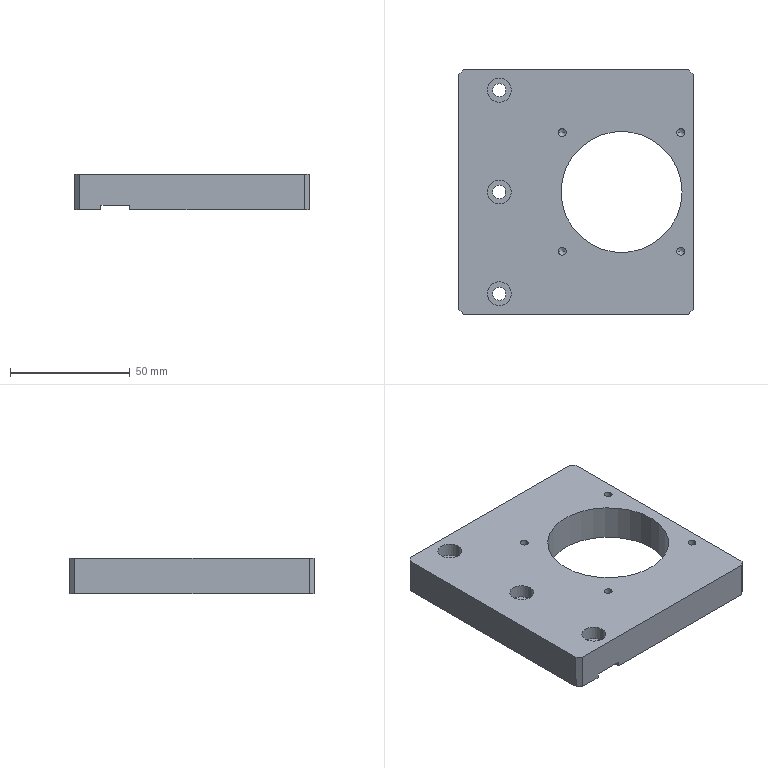Part | SolidWorks | features BaseBody 1 | 1 solid | 55 faces | box 98 x 102 x 15 mm | volume 114752 mm3 | cylinder 26 | plane 17 | cone 12 | commonest cylinder face diameters 3.3 x8 5.5 x6 10 x6 4.2 x4 50.5 x2
STEP:
#1=CARTESIAN_POINT('',(-37.,42.5,7.3));
#2=VERTEX_POINT('',#1);
#3=CARTESIAN_POINT('',(-27.,42.5,7.3));
#4=VERTEX_POINT('',#3);
#5=CARTESIAN_POINT('',(-32.,42.5,7.3));
#6=DIRECTION('',(0.,0.,1.));
#7=DIRECTION('',(1.,0.,0.));
#8=AXIS2_PLACEMENT_3D('',#5,#6,#7);
#9=CIRCLE('',#8,5.);
#10=EDGE_CURVE('',#2,#4,#9,.T.);
#11=ORIENTED_EDGE('',*,*,#10,.F.);
#12=CARTESIAN_POINT('',(-37.,42.5,13.));
#13=VERTEX_POINT('',#12);
#14=CARTESIAN_POINT('',(-37.,42.5,13.));
#15=DIRECTION('',(0.,0.,1.));
#16=VECTOR('',#15,1000.);
#17=LINE('',#14,#16);
#18=EDGE_CURVE('',#2,#13,#17,.T.);
#19=ORIENTED_EDGE('',*,*,#18,.T.);
#20=CARTESIAN_POINT('',(-27.,42.5,13.));
#21=VERTEX_POINT('',#20);
#22=CARTESIAN_POINT('',(-32.,42.5,13.));
#23=DIRECTION('',(0.,0.,-1.));
#24=DIRECTION('',(1.,0.,0.));
#25=AXIS2_PLACEMENT_3D('',#22,#23,#24);
#26=CIRCLE('',#25,5.);
#27=EDGE_CURVE('',#21,#13,#26,.T.);
#28=ORIENTED_EDGE('',*,*,#27,.F.);
#29=CARTESIAN_POINT('',(-27.,42.5,13.));
#30=DIRECTION('',(0.,0.,1.));
#31=VECTOR('',#30,1000.);
#32=LINE('',#29,#31);
#33=EDGE_CURVE('',#4,#21,#32,.T.);
#34=ORIENTED_EDGE('',*,*,#33,.F.);
#35=EDGE_LOOP('',(#11,#19,#28,#34));
#36=FACE_OUTER_BOUND('',#35,.T.);
#37=CARTESIAN_POINT('',(-32.,42.5,13.));
#38=DIRECTION('',(0.,0.,1.));
#39=DIRECTION('',(1.,0.,0.));
#40=AXIS2_PLACEMENT_3D('',#37,#38,#39);
#41=CYLINDRICAL_SURFACE('',#40,5.);
#42=ADVANCED_FACE('',(#36),#41,.F.);
#43=CARTESIAN_POINT('',(-37.,0.,7.3));
#44=VERTEX_POINT('',#43);
#45=CARTESIAN_POINT('',(-27.,0.,7.3));
#46=VERTEX_POINT('',#45);
#47=CARTESIAN_POINT('',(-32.,0.,7.3));
#48=DIRECTION('',(0.,0.,1.));
#49=DIRECTION('',(1.,0.,0.));
#50=AXIS2_PLACEMENT_3D('',#47,#48,#49);
#51=CIRCLE('',#50,5.);
#52=EDGE_CURVE('',#44,#46,#51,.T.);
#53=ORIENTED_EDGE('',*,*,#52,.F.);
#54=CARTESIAN_POINT('',(-37.,0.,13.));
#55=VERTEX_POINT('',#54);
#56=CARTESIAN_POINT('',(-37.,0.,13.));
#57=DIRECTION('',(0.,0.,1.));
#58=VECTOR('',#57,1000.);
#59=LINE('',#56,#58);
#60=EDGE_CURVE('',#44,#55,#59,.T.);
#61=ORIENTED_EDGE('',*,*,#60,.T.);
#62=CARTESIAN_POINT('',(-27.,0.,13.));
#63=VERTEX_POINT('',#62);
#64=CARTESIAN_POINT('',(-32.,0.,13.));
#65=DIRECTION('',(0.,0.,-1.));
#66=DIRECTION('',(1.,0.,0.));
#67=AXIS2_PLACEMENT_3D('',#64,#65,#66);
#68=CIRCLE('',#67,5.);
#69=EDGE_CURVE('',#63,#55,#68,.T.);
#70=ORIENTED_EDGE('',*,*,#69,.F.);
#71=CARTESIAN_POINT('',(-27.,0.,13.));
#72=DIRECTION('',(0.,0.,1.));
#73=VECTOR('',#72,1000.);
#74=LINE('',#71,#73);
#75=EDGE_CURVE('',#46,#63,#74,.T.);
#76=ORIENTED_EDGE('',*,*,#75,.F.);
#77=EDGE_LOOP('',(#53,#61,#70,#76));
#78=FACE_OUTER_BOUND('',#77,.T.);
#79=CARTESIAN_POINT('',(-32.,0.,13.));
#80=DIRECTION('',(0.,0.,1.));
#81=DIRECTION('',(1.,0.,0.));
#82=AXIS2_PLACEMENT_3D('',#79,#80,#81);
#83=CYLINDRICAL_SURFACE('',#82,5.);
#84=ADVANCED_FACE('',(#78),#83,.F.);
#85=CARTESIAN_POINT('',(-37.,-42.5,7.3));
#86=VERTEX_POINT('',#85);
#87=CARTESIAN_POINT('',(-27.,-42.5,7.3));
#88=VERTEX_POINT('',#87);
#89=CARTESIAN_POINT('',(-32.,-42.5,7.3));
#90=DIRECTION('',(0.,0.,1.));
#91=DIRECTION('',(1.,0.,0.));
#92=AXIS2_PLACEMENT_3D('',#89,#90,#91);
#93=CIRCLE('',#92,5.);
#94=EDGE_CURVE('',#86,#88,#93,.T.);
#95=ORIENTED_EDGE('',*,*,#94,.F.);
#96=CARTESIAN_POINT('',(-37.,-42.5,13.));
#97=VERTEX_POINT('',#96);
#98=CARTESIAN_POINT('',(-37.,-42.5,13.));
#99=DIRECTION('',(0.,0.,1.));
#100=VECTOR('',#99,1000.);
#101=LINE('',#98,#100);
#102=EDGE_CURVE('',#86,#97,#101,.T.);
#103=ORIENTED_EDGE('',*,*,#102,.T.);
#104=CARTESIAN_POINT('',(-27.,-42.5,13.));
#105=VERTEX_POINT('',#104);
#106=CARTESIAN_POINT('',(-32.,-42.5,13.));
#107=DIRECTION('',(0.,0.,-1.));
#108=DIRECTION('',(1.,0.,0.));
#109=AXIS2_PLACEMENT_3D('',#106,#107,#108);
#110=CIRCLE('',#109,5.);
#111=EDGE_CURVE('',#105,#97,#110,.T.);
#112=ORIENTED_EDGE('',*,*,#111,.F.);
#113=CARTESIAN_POINT('',(-27.,-42.5,13.));
#114=DIRECTION('',(0.,0.,1.));
#115=VECTOR('',#114,1000.);
#116=LINE('',#113,#115);
#117=EDGE_CURVE('',#88,#105,#116,.T.);
#118=ORIENTED_EDGE('',*,*,#117,.F.);
#119=EDGE_LOOP('',(#95,#103,#112,#118));
#120=FACE_OUTER_BOUND('',#119,.T.);
#121=CARTESIAN_POINT('',(-32.,-42.5,13.));
#122=DIRECTION('',(0.,0.,1.));
#123=DIRECTION('',(1.,0.,0.));
#124=AXIS2_PLACEMENT_3D('',#121,#122,#123);
#125=CYLINDRICAL_SURFACE('',#124,5.);
#126=ADVANCED_FACE('',(#120),#125,.F.);
#127=CARTESIAN_POINT('',(44.25,0.,13.));
#128=VERTEX_POINT('',#127);
#129=CARTESIAN_POINT('',(-6.25,0.,13.));
#130=VERTEX_POINT('',#129);
#131=CARTESIAN_POINT('',(19.,0.,13.));
#132=DIRECTION('',(0.,0.,-1.));
#133=DIRECTION('',(-1.,0.,0.));
#134=AXIS2_PLACEMENT_3D('',#131,#132,#133);
#135=CIRCLE('',#134,25.25);
#136=EDGE_CURVE('',#128,#130,#135,.T.);
#137=ORIENTED_EDGE('',*,*,#136,.F.);
#138=CARTESIAN_POINT('',(44.25,0.,-2.));
#139=VERTEX_POINT('',#138);
#140=CARTESIAN_POINT('',(44.25,0.,13.));
#141=DIRECTION('',(0.,0.,-1.));
#142=VECTOR('',#141,1000.);
#143=LINE('',#140,#142);
#144=EDGE_CURVE('',#128,#139,#143,.T.);
#145=ORIENTED_EDGE('',*,*,#144,.T.);
#146=CARTESIAN_POINT('',(-6.25,0.,-2.));
#147=VERTEX_POINT('',#146);
#148=CARTESIAN_POINT('',(19.,0.,-2.));
#149=DIRECTION('',(0.,0.,1.));
#150=DIRECTION('',(-1.,0.,0.));
#151=AXIS2_PLACEMENT_3D('',#148,#149,#150);
#152=CIRCLE('',#151,25.25);
#153=EDGE_CURVE('',#147,#139,#152,.T.);
#154=ORIENTED_EDGE('',*,*,#153,.F.);
#155=CARTESIAN_POINT('',(-6.25,0.,13.));
#156=DIRECTION('',(0.,0.,-1.));
#157=VECTOR('',#156,1000.);
#158=LINE('',#155,#157);
#159=EDGE_CURVE('',#130,#147,#158,.T.);
#160=ORIENTED_EDGE('',*,*,#159,.F.);
#161=EDGE_LOOP('',(#137,#145,#154,#160));
#162=FACE_OUTER_BOUND('',#161,.T.);
#163=CARTESIAN_POINT('',(19.,0.,13.));
#164=DIRECTION('',(0.,0.,-1.));
#165=DIRECTION('',(-1.,0.,0.));
#166=AXIS2_PLACEMENT_3D('',#163,#164,#165);
#167=CYLINDRICAL_SURFACE('',#166,25.25);
#168=ADVANCED_FACE('',(#162),#167,.F.);
#169=CARTESIAN_POINT('',(42.1,-24.75,2.9));
#170=VERTEX_POINT('',#169);
#171=CARTESIAN_POINT('',(45.4,-24.75,2.9));
#172=VERTEX_POINT('',#171);
#173=CARTESIAN_POINT('',(43.75,-24.75,2.9));
#174=DIRECTION('',(0.,0.,1.));
#175=DIRECTION('',(1.,0.,0.));
#176=AXIS2_PLACEMENT_3D('',#173,#174,#175);
#177=CIRCLE('',#176,1.65);
#178=EDGE_CURVE('',#170,#172,#177,.T.);
#179=ORIENTED_EDGE('',*,*,#178,.F.);
#180=CARTESIAN_POINT('',(42.1,-24.75,13.));
#181=VERTEX_POINT('',#180);
#182=CARTESIAN_POINT('',(42.1,-24.75,13.));
#183=DIRECTION('',(0.,0.,1.));
#184=VECTOR('',#183,1000.);
#185=LINE('',#182,#184);
#186=EDGE_CURVE('',#170,#181,#185,.T.);
#187=ORIENTED_EDGE('',*,*,#186,.T.);
#188=CARTESIAN_POINT('',(45.4,-24.75,13.));
#189=VERTEX_POINT('',#188);
#190=CARTESIAN_POINT('',(43.75,-24.75,13.));
#191=DIRECTION('',(0.,0.,-1.));
#192=DIRECTION('',(1.,0.,0.));
#193=AXIS2_PLACEMENT_3D('',#190,#191,#192);
#194=CIRCLE('',#193,1.65);
#195=EDGE_CURVE('',#189,#181,#194,.T.);
#196=ORIENTED_EDGE('',*,*,#195,.F.);
#197=CARTESIAN_POINT('',(45.4,-24.75,13.));
#198=DIRECTION('',(0.,0.,1.));
#199=VECTOR('',#198,1000.);
#200=LINE('',#197,#199);
#201=EDGE_CURVE('',#172,#189,#200,.T.);
#202=ORIENTED_EDGE('',*,*,#201,.F.);
#203=EDGE_LOOP('',(#179,#187,#196,#202));
#204=FACE_OUTER_BOUND('',#203,.T.);
#205=CARTESIAN_POINT('',(43.75,-24.75,13.));
#206=DIRECTION('',(0.,0.,1.));
#207=DIRECTION('',(1.,0.,0.));
#208=AXIS2_PLACEMENT_3D('',#205,#206,#207);
#209=CYLINDRICAL_SURFACE('',#208,1.65);
#210=ADVANCED_FACE('',(#204),#209,.F.);
#211=CARTESIAN_POINT('',(-7.4,-24.75,2.9));
#212=VERTEX_POINT('',#211);
#213=CARTESIAN_POINT('',(-4.1,-24.75,2.9));
#214=VERTEX_POINT('',#213);
#215=CARTESIAN_POINT('',(-5.75,-24.75,2.9));
#216=DIRECTION('',(0.,0.,1.));
#217=DIRECTION('',(1.,0.,0.));
#218=AXIS2_PLACEMENT_3D('',#215,#216,#217);
#219=CIRCLE('',#218,1.65);
#220=EDGE_CURVE('',#212,#214,#219,.T.);
#221=ORIENTED_EDGE('',*,*,#220,.F.);
#222=CARTESIAN_POINT('',(-7.4,-24.75,13.));
#223=VERTEX_POINT('',#222);
#224=CARTESIAN_POINT('',(-7.4,-24.75,13.));
#225=DIRECTION('',(0.,0.,1.));
#226=VECTOR('',#225,1000.);
#227=LINE('',#224,#226);
#228=EDGE_CURVE('',#212,#223,#227,.T.);
#229=ORIENTED_EDGE('',*,*,#228,.T.);
#230=CARTESIAN_POINT('',(-4.1,-24.75,13.));
#231=VERTEX_POINT('',#230);
#232=CARTESIAN_POINT('',(-5.75,-24.75,13.));
#233=DIRECTION('',(0.,0.,-1.));
#234=DIRECTION('',(1.,0.,0.));
#235=AXIS2_PLACEMENT_3D('',#232,#233,#234);
#236=CIRCLE('',#235,1.65);
#237=EDGE_CURVE('',#231,#223,#236,.T.);
#238=ORIENTED_EDGE('',*,*,#237,.F.);
#239=CARTESIAN_POINT('',(-4.1,-24.75,13.));
#240=DIRECTION('',(0.,0.,1.));
#241=VECTOR('',#240,1000.);
#242=LINE('',#239,#241);
#243=EDGE_CURVE('',#214,#231,#242,.T.);
#244=ORIENTED_EDGE('',*,*,#243,.F.);
#245=EDGE_LOOP('',(#221,#229,#238,#244));
#246=FACE_OUTER_BOUND('',#245,.T.);
#247=CARTESIAN_POINT('',(-5.75,-24.75,13.));
#248=DIRECTION('',(0.,0.,1.));
#249=DIRECTION('',(1.,0.,0.));
#250=AXIS2_PLACEMENT_3D('',#247,#248,#249);
#251=CYLINDRICAL_SURFACE('',#250,1.65);
#252=ADVANCED_FACE('',(#246),#251,.F.);
#253=CARTESIAN_POINT('',(-7.4,24.75,2.9));
#254=VERTEX_POINT('',#253);
#255=CARTESIAN_POINT('',(-4.1,24.75,2.9));
#256=VERTEX_POINT('',#255);
#257=CARTESIAN_POINT('',(-5.75,24.75,2.9));
#258=DIRECTION('',(0.,0.,1.));
#259=DIRECTION('',(1.,0.,0.));
#260=AXIS2_PLACEMENT_3D('',#257,#258,#259);
#261=CIRCLE('',#260,1.65);
#262=EDGE_CURVE('',#254,#256,#261,.T.);
#263=ORIENTED_EDGE('',*,*,#262,.F.);
#264=CARTESIAN_POINT('',(-7.4,24.75,13.));
#265=VERTEX_POINT('',#264);
#266=CARTESIAN_POINT('',(-7.4,24.75,13.));
#267=DIRECTION('',(0.,0.,1.));
#268=VECTOR('',#267,1000.);
#269=LINE('',#266,#268);
#270=EDGE_CURVE('',#254,#265,#269,.T.);
#271=ORIENTED_EDGE('',*,*,#270,.T.);
#272=CARTESIAN_POINT('',(-4.1,24.75,13.));
#273=VERTEX_POINT('',#272);
#274=CARTESIAN_POINT('',(-5.75,24.75,13.));
#275=DIRECTION('',(0.,0.,-1.));
#276=DIRECTION('',(1.,0.,0.));
#277=AXIS2_PLACEMENT_3D('',#274,#275,#276);
#278=CIRCLE('',#277,1.65);
#279=EDGE_CURVE('',#273,#265,#278,.T.);
#280=ORIENTED_EDGE('',*,*,#279,.F.);
#281=CARTESIAN_POINT('',(-4.1,24.75,13.));
#282=DIRECTION('',(0.,0.,1.));
#283=VECTOR('',#282,1000.);
#284=LINE('',#281,#283);
#285=EDGE_CURVE('',#256,#273,#284,.T.);
#286=ORIENTED_EDGE('',*,*,#285,.F.);
#287=EDGE_LOOP('',(#263,#271,#280,#286));
#288=FACE_OUTER_BOUND('',#287,.T.);
#289=CARTESIAN_POINT('',(-5.75,24.75,13.));
#290=DIRECTION('',(0.,0.,1.));
#291=DIRECTION('',(1.,0.,0.));
#292=AXIS2_PLACEMENT_3D('',#289,#290,#291);
#293=CYLINDRICAL_SURFACE('',#292,1.65);
#294=ADVANCED_FACE('',(#288),#293,.F.);
#295=CARTESIAN_POINT('',(42.1,24.75,2.9));
#296=VERTEX_POINT('',#295);
#297=CARTESIAN_POINT('',(45.4,24.75,2.9));
#298=VERTEX_POINT('',#297);
#299=CARTESIAN_POINT('',(43.75,24.75,2.9));
#300=DIRECTION('',(0.,0.,1.));
#301=DIRECTION('',(1.,0.,0.));
#302=AXIS2_PLACEMENT_3D('',#299,#300,#301);
#303=CIRCLE('',#302,1.65);
#304=EDGE_CURVE('',#296,#298,#303,.T.);
#305=ORIENTED_EDGE('',*,*,#304,.F.);
#306=CARTESIAN_POINT('',(42.1,24.75,13.));
#307=VERTEX_POINT('',#306);
#308=CARTESIAN_POINT('',(42.1,24.75,13.));
#309=DIRECTION('',(0.,0.,1.));
#310=VECTOR('',#309,1000.);
#311=LINE('',#308,#310);
#312=EDGE_CURVE('',#296,#307,#311,.T.);
#313=ORIENTED_EDGE('',*,*,#312,.T.);
#314=CARTESIAN_POINT('',(45.4,24.75,13.));
#315=VERTEX_POINT('',#314);
#316=CARTESIAN_POINT('',(43.75,24.75,13.));
#317=DIRECTION('',(0.,0.,-1.));
#318=DIRECTION('',(1.,0.,0.));
#319=AXIS2_PLACEMENT_3D('',#316,#317,#318);
#320=CIRCLE('',#319,1.65);
#321=EDGE_CURVE('',#315,#307,#320,.T.);
#322=ORIENTED_EDGE('',*,*,#321,.F.);
#323=CARTESIAN_POINT('',(45.4,24.75,13.));
#324=DIRECTION('',(0.,0.,1.));
#325=VECTOR('',#324,1000.);
#326=LINE('',#323,#325);
#327=EDGE_CURVE('',#298,#315,#326,.T.);
#328=ORIENTED_EDGE('',*,*,#327,.F.);
#329=EDGE_LOOP('',(#305,#313,#322,#328));
#330=FACE_OUTER_BOUND('',#329,.T.);
#331=CARTESIAN_POINT('',(43.75,24.75,13.));
#332=DIRECTION('',(0.,0.,1.));
#333=DIRECTION('',(1.,0.,0.));
#334=AXIS2_PLACEMENT_3D('',#331,#332,#333);
#335=CYLINDRICAL_SURFACE('',#334,1.65);
#336=ADVANCED_FACE('',(#330),#335,.F.);
#337=CARTESIAN_POINT('',(36.6,-33.,7.6));
#338=VERTEX_POINT('',#337);
#339=CARTESIAN_POINT('',(36.6,-33.,3.4));
#340=VERTEX_POINT('',#339);
#341=CARTESIAN_POINT('',(36.6,-33.,5.5));
#342=DIRECTION('',(1.,0.,0.));
#343=DIRECTION('',(0.,0.,-1.));
#344=AXIS2_PLACEMENT_3D('',#341,#342,#343);
#345=CIRCLE('',#344,2.1);
#346=EDGE_CURVE('',#338,#340,#345,.T.);
#347=ORIENTED_EDGE('',*,*,#346,.F.);
#348=CARTESIAN_POINT('',(49.,-33.,7.6));
#349=VERTEX_POINT('',#348);
#350=CARTESIAN_POINT('',(49.,-33.,7.6));
#351=DIRECTION('',(1.,0.,0.));
#352=VECTOR('',#351,1000.);
#353=LINE('',#350,#352);
#354=EDGE_CURVE('',#338,#349,#353,.T.);
#355=ORIENTED_EDGE('',*,*,#354,.T.);
#356=CARTESIAN_POINT('',(49.,-33.,3.4));
#357=VERTEX_POINT('',#356);
#358=CARTESIAN_POINT('',(49.,-33.,5.5));
#359=DIRECTION('',(1.,0.,0.));
#360=DIRECTION('',(0.,0.,-1.));
#361=AXIS2_PLACEMENT_3D('',#358,#359,#360);
#362=CIRCLE('',#361,2.1);
#363=EDGE_CURVE('',#349,#357,#362,.T.);
#364=ORIENTED_EDGE('',*,*,#363,.T.);
#365=CARTESIAN_POINT('',(49.,-33.,3.4));
#366=DIRECTION('',(1.,0.,0.));
#367=VECTOR('',#366,1000.);
#368=LINE('',#365,#367);
#369=EDGE_CURVE('',#340,#357,#368,.T.);
#370=ORIENTED_EDGE('',*,*,#369,.F.);
#371=EDGE_LOOP('',(#347,#355,#364,#370));
#372=FACE_OUTER_BOUND('',#371,.T.);
#373=CARTESIAN_POINT('',(49.,-33.,5.5));
#374=DIRECTION('',(1.,0.,0.));
#375=DIRECTION('',(0.,0.,-1.));
#376=AXIS2_PLACEMENT_3D('',#373,#374,#375);
#377=CYLINDRICAL_SURFACE('',#376,2.1);
#378=ADVANCED_FACE('',(#372),#377,.F.);
#379=CARTESIAN_POINT('',(36.6,33.,7.6));
#380=VERTEX_POINT('',#379);
#381=CARTESIAN_POINT('',(36.6,33.,3.4));
#382=VERTEX_POINT('',#381);
#383=CARTESIAN_POINT('',(36.6,33.,5.5));
#384=DIRECTION('',(1.,0.,0.));
#385=DIRECTION('',(0.,0.,-1.));
#386=AXIS2_PLACEMENT_3D('',#383,#384,#385);
#387=CIRCLE('',#386,2.1);
#388=EDGE_CURVE('',#380,#382,#387,.T.);
#389=ORIENTED_EDGE('',*,*,#388,.F.);
#390=CARTESIAN_POINT('',(49.,33.,7.6));
#391=VERTEX_POINT('',#390);
#392=CARTESIAN_POINT('',(49.,33.,7.6));
#393=DIRECTION('',(1.,0.,0.));
#394=VECTOR('',#393,1000.);
#395=LINE('',#392,#394);
#396=EDGE_CURVE('',#380,#391,#395,.T.);
#397=ORIENTED_EDGE('',*,*,#396,.T.);
#398=CARTESIAN_POINT('',(49.,33.,3.4));
#399=VERTEX_POINT('',#398);
#400=CARTESIAN_POINT('',(49.,33.,5.5));
#401=DIRECTION('',(1.,0.,0.));
#402=DIRECTION('',(0.,0.,-1.));
#403=AXIS2_PLACEMENT_3D('',#400,#401,#402);
#404=CIRCLE('',#403,2.1);
#405=EDGE_CURVE('',#391,#399,#404,.T.);
#406=ORIENTED_EDGE('',*,*,#405,.T.);
#407=CARTESIAN_POINT('',(49.,33.,3.4));
#408=DIRECTION('',(1.,0.,0.));
#409=VECTOR('',#408,1000.);
#410=LINE('',#407,#409);
#411=EDGE_CURVE('',#382,#399,#410,.T.);
#412=ORIENTED_EDGE('',*,*,#411,.F.);
#413=EDGE_LOOP('',(#389,#397,#406,#412));
#414=FACE_OUTER_BOUND('',#413,.T.);
#415=CARTESIAN_POINT('',(49.,33.,5.5));
#416=DIRECTION('',(1.,0.,0.));
#417=DIRECTION('',(0.,0.,-1.));
#418=AXIS2_PLACEMENT_3D('',#415,#416,#417);
#419=CYLINDRICAL_SURFACE('',#418,2.1);
#420=ADVANCED_FACE('',(#414),#419,.F.);
#421=CARTESIAN_POINT('',(43.75,-24.75,1.909));
#422=VERTEX_POINT('',#421);
#423=CARTESIAN_POINT('',(45.4,-24.75,2.9));
#424=DIRECTION('',(0.8572,0.,0.515));
#425=VECTOR('',#424,1000.);
#426=LINE('',#423,#425);
#427=EDGE_CURVE('',#422,#172,#426,.T.);
#428=ORIENTED_EDGE('',*,*,#427,.F.);
#429=CARTESIAN_POINT('',(42.1,-24.75,2.9));
#430=DIRECTION('',(-0.8572,0.,0.515));
#431=VECTOR('',#430,1000.);
#432=LINE('',#429,#431);
#433=EDGE_CURVE('',#422,#170,#432,.T.);
#434=ORIENTED_EDGE('',*,*,#433,.T.);
#435=ORIENTED_EDGE('',*,*,#178,.T.);
#436=EDGE_LOOP('',(#428,#434,#435));
#437=FACE_OUTER_BOUND('',#436,.T.);
#438=CARTESIAN_POINT('',(43.75,-24.75,2.9));
#439=DIRECTION('',(0.,0.,1.));
#440=DIRECTION('',(1.,0.,0.));
#441=AXIS2_PLACEMENT_3D('',#438,#439,#440);
#442=CONICAL_SURFACE('',#441,1.65,1.03);
#443=ADVANCED_FACE('',(#437),#442,.F.);
#444=CARTESIAN_POINT('',(-5.75,-24.75,1.909));
#445=VERTEX_POINT('',#444);
#446=CARTESIAN_POINT('',(-4.1,-24.75,2.9));
#447=DIRECTION('',(0.8572,0.,0.515));
#448=VECTOR('',#447,1000.);
#449=LINE('',#446,#448);
#450=EDGE_CURVE('',#445,#214,#449,.T.);
#451=ORIENTED_EDGE('',*,*,#450,.F.);
#452=CARTESIAN_POINT('',(-7.4,-24.75,2.9));
#453=DIRECTION('',(-0.8572,0.,0.515));
#454=VECTOR('',#453,1000.);
#455=LINE('',#452,#454);
#456=EDGE_CURVE('',#445,#212,#455,.T.);
#457=ORIENTED_EDGE('',*,*,#456,.T.);
#458=ORIENTED_EDGE('',*,*,#220,.T.);
#459=EDGE_LOOP('',(#451,#457,#458));
#460=FACE_OUTER_BOUND('',#459,.T.);
#461=CARTESIAN_POINT('',(-5.75,-24.75,2.9));
#462=DIRECTION('',(0.,0.,1.));
#463=DIRECTION('',(1.,0.,0.));
#464=AXIS2_PLACEMENT_3D('',#461,#462,#463);
#465=CONICAL_SURFACE('',#464,1.65,1.03);
#466=ADVANCED_FACE('',(#460),#465,.F.);
#467=CARTESIAN_POINT('',(-5.75,24.75,1.909));
#468=VERTEX_POINT('',#467);
#469=CARTESIAN_POINT('',(-4.1,24.75,2.9));
#470=DIRECTION('',(0.8572,0.,0.515));
#471=VECTOR('',#470,1000.);
#472=LINE('',#469,#471);
#473=EDGE_CURVE('',#468,#256,#472,.T.);
#474=ORIENTED_EDGE('',*,*,#473,.F.);
#475=CARTESIAN_POINT('',(-7.4,24.75,2.9));
#476=DIRECTION('',(-0.8572,0.,0.515));
#477=VECTOR('',#476,1000.);
#478=LINE('',#475,#477);
#479=EDGE_CURVE('',#468,#254,#478,.T.);
#480=ORIENTED_EDGE('',*,*,#479,.T.);
#481=ORIENTED_EDGE('',*,*,#262,.T.);
#482=EDGE_LOOP('',(#474,#480,#481));
#483=FACE_OUTER_BOUND('',#482,.T.);
#484=CARTESIAN_POINT('',(-5.75,24.75,2.9));
#485=DIRECTION('',(0.,0.,1.));
#486=DIRECTION('',(1.,0.,0.));
#487=AXIS2_PLACEMENT_3D('',#484,#485,#486);
#488=CONICAL_SURFACE('',#487,1.65,1.03);
#489=ADVANCED_FACE('',(#483),#488,.F.);
#490=CARTESIAN_POINT('',(43.75,24.75,1.909));
#491=VERTEX_POINT('',#490);
#492=CARTESIAN_POINT('',(45.4,24.75,2.9));
#493=DIRECTION('',(0.8572,0.,0.515));
#494=VECTOR('',#493,1000.);
#495=LINE('',#492,#494);
#496=EDGE_CURVE('',#491,#298,#495,.T.);
#497=ORIENTED_EDGE('',*,*,#496,.F.);
#498=CARTESIAN_POINT('',(42.1,24.75,2.9));
#499=DIRECTION('',(-0.8572,0.,0.515));
#500=VECTOR('',#499,1000.);
#501=LINE('',#498,#500);
#502=EDGE_CURVE('',#491,#296,#501,.T.);
#503=ORIENTED_EDGE('',*,*,#502,.T.);
#504=ORIENTED_EDGE('',*,*,#304,.T.);
#505=EDGE_LOOP('',(#497,#503,#504));
#506=FACE_OUTER_BOUND('',#505,.T.);
#507=CARTESIAN_POINT('',(43.75,24.75,2.9));
#508=DIRECTION('',(0.,0.,1.));
#509=DIRECTION('',(1.,0.,0.));
#510=AXIS2_PLACEMENT_3D('',#507,#508,#509);
#511=CONICAL_SURFACE('',#510,1.65,1.03);
#512=ADVANCED_FACE('',(#506),#511,.F.);
#513=CARTESIAN_POINT('',(-29.25,42.5,0.));
#514=VERTEX_POINT('',#513);
#515=CARTESIAN_POINT('',(-34.75,42.5,0.));
#516=VERTEX_POINT('',#515);
#517=CARTESIAN_POINT('',(-32.,42.5,0.));
#518=DIRECTION('',(0.,0.,-1.));
#519=DIRECTION('',(1.,0.,0.));
#520=AXIS2_PLACEMENT_3D('',#517,#518,#519);
#521=CIRCLE('',#520,2.75);
#522=EDGE_CURVE('',#514,#516,#521,.T.);
#523=ORIENTED_EDGE('',*,*,#522,.T.);
#524=CARTESIAN_POINT('',(-34.75,42.5,7.3));
#525=VERTEX_POINT('',#524);
#526=CARTESIAN_POINT('',(-34.75,42.5,13.));
#527=DIRECTION('',(0.,0.,1.));
#528=VECTOR('',#527,1000.);
#529=LINE('',#526,#528);
#530=EDGE_CURVE('',#516,#525,#529,.T.);
#531=ORIENTED_EDGE('',*,*,#530,.T.);
#532=CARTESIAN_POINT('',(-29.25,42.5,7.3));
#533=VERTEX_POINT('',#532);
#534=CARTESIAN_POINT('',(-32.,42.5,7.3));
#535=DIRECTION('',(0.,0.,1.));
#536=DIRECTION('',(1.,0.,0.));
#537=AXIS2_PLACEMENT_3D('',#534,#535,#536);
#538=CIRCLE('',#537,2.75);
#539=EDGE_CURVE('',#525,#533,#538,.T.);
#540=ORIENTED_EDGE('',*,*,#539,.T.);
#541=CARTESIAN_POINT('',(-29.25,42.5,13.));
#542=DIRECTION('',(0.,0.,1.));
#543=VECTOR('',#542,1000.);
#544=LINE('',#541,#543);
#545=EDGE_CURVE('',#514,#533,#544,.T.);
#546=ORIENTED_EDGE('',*,*,#545,.F.);
#547=EDGE_LOOP('',(#523,#531,#540,#546));
#548=FACE_OUTER_BOUND('',#547,.T.);
#549=CARTESIAN_POINT('',(-32.,42.5,13.));
#550=DIRECTION('',(0.,0.,1.));
#551=DIRECTION('',(1.,0.,0.));
#552=AXIS2_PLACEMENT_3D('',#549,#550,#551);
#553=CYLINDRICAL_SURFACE('',#552,2.75);
#554=ADVANCED_FACE('',(#548),#553,.F.);
#555=CARTESIAN_POINT('',(-29.25,0.,0.));
#556=VERTEX_POINT('',#555);
#557=CARTESIAN_POINT('',(-34.75,0.,0.));
#558=VERTEX_POINT('',#557);
#559=CARTESIAN_POINT('',(-32.,0.,0.));
#560=DIRECTION('',(0.,0.,-1.));
#561=DIRECTION('',(1.,0.,0.));
#562=AXIS2_PLACEMENT_3D('',#559,#560,#561);
#563=CIRCLE('',#562,2.75);
#564=EDGE_CURVE('',#556,#558,#563,.T.);
#565=ORIENTED_EDGE('',*,*,#564,.T.);
#566=CARTESIAN_POINT('',(-34.75,0.,7.3));
#567=VERTEX_POINT('',#566);
#568=CARTESIAN_POINT('',(-34.75,0.,13.));
#569=DIRECTION('',(0.,0.,1.));
#570=VECTOR('',#569,1000.);
#571=LINE('',#568,#570);
#572=EDGE_CURVE('',#558,#567,#571,.T.);
#573=ORIENTED_EDGE('',*,*,#572,.T.);
#574=CARTESIAN_POINT('',(-29.25,0.,7.3));
#575=VERTEX_POINT('',#574);
#576=CARTESIAN_POINT('',(-32.,0.,7.3));
#577=DIRECTION('',(0.,0.,1.));
#578=DIRECTION('',(1.,0.,0.));
#579=AXIS2_PLACEMENT_3D('',#576,#577,#578);
#580=CIRCLE('',#579,2.75);
#581=EDGE_CURVE('',#567,#575,#580,.T.);
#582=ORIENTED_EDGE('',*,*,#581,.T.);
#583=CARTESIAN_POINT('',(-29.25,0.,13.));
#584=DIRECTION('',(0.,0.,1.));
#585=VECTOR('',#584,1000.);
#586=LINE('',#583,#585);
#587=EDGE_CURVE('',#556,#575,#586,.T.);
#588=ORIENTED_EDGE('',*,*,#587,.F.);
#589=EDGE_LOOP('',(#565,#573,#582,#588));
#590=FACE_OUTER_BOUND('',#589,.T.);
#591=CARTESIAN_POINT('',(-32.,0.,13.));
#592=DIRECTION('',(0.,0.,1.));
#593=DIRECTION('',(1.,0.,0.));
#594=AXIS2_PLACEMENT_3D('',#591,#592,#593);
#595=CYLINDRICAL_SURFACE('',#594,2.75);
#596=ADVANCED_FACE('',(#590),#595,.F.);
#597=CARTESIAN_POINT('',(-29.25,-42.5,0.));
#598=VERTEX_POINT('',#597);
#599=CARTESIAN_POINT('',(-34.75,-42.5,0.));
#600=VERTEX_POINT('',#599);
#601=CARTESIAN_POINT('',(-32.,-42.5,0.));
#602=DIRECTION('',(0.,0.,-1.));
#603=DIRECTION('',(1.,0.,0.));
#604=AXIS2_PLACEMENT_3D('',#601,#602,#603);
#605=CIRCLE('',#604,2.75);
#606=EDGE_CURVE('',#598,#600,#605,.T.);
#607=ORIENTED_EDGE('',*,*,#606,.T.);
#608=CARTESIAN_POINT('',(-34.75,-42.5,7.3));
#609=VERTEX_POINT('',#608);
#610=CARTESIAN_POINT('',(-34.75,-42.5,13.));
#611=DIRECTION('',(0.,0.,1.));
#612=VECTOR('',#611,1000.);
#613=LINE('',#610,#612);
#614=EDGE_CURVE('',#600,#609,#613,.T.);
#615=ORIENTED_EDGE('',*,*,#614,.T.);
#616=CARTESIAN_POINT('',(-29.25,-42.5,7.3));
#617=VERTEX_POINT('',#616);
#618=CARTESIAN_POINT('',(-32.,-42.5,7.3));
#619=DIRECTION('',(0.,0.,1.));
#620=DIRECTION('',(1.,0.,0.));
#621=AXIS2_PLACEMENT_3D('',#618,#619,#620);
#622=CIRCLE('',#621,2.75);
#623=EDGE_CURVE('',#609,#617,#622,.T.);
#624=ORIENTED_EDGE('',*,*,#623,.T.);
#625=CARTESIAN_POINT('',(-29.25,-42.5,13.));
#626=DIRECTION('',(0.,0.,1.));
#627=VECTOR('',#626,1000.);
#628=LINE('',#625,#627);
#629=EDGE_CURVE('',#598,#617,#628,.T.);
#630=ORIENTED_EDGE('',*,*,#629,.F.);
#631=EDGE_LOOP('',(#607,#615,#624,#630));
#632=FACE_OUTER_BOUND('',#631,.T.);
#633=CARTESIAN_POINT('',(-32.,-42.5,13.));
#634=DIRECTION('',(0.,0.,1.));
#635=DIRECTION('',(1.,0.,0.));
#636=AXIS2_PLACEMENT_3D('',#633,#634,#635);
#637=CYLINDRICAL_SURFACE('',#636,2.75);
#638=ADVANCED_FACE('',(#632),#637,.F.);
#639=CARTESIAN_POINT('',(35.338,-33.,5.5));
#640=VERTEX_POINT('',#639);
#641=CARTESIAN_POINT('',(36.6,-33.,3.4));
#642=DIRECTION('',(0.515,0.,-0.8572));
#643=VECTOR('',#642,1000.);
#644=LINE('',#641,#643);
#645=EDGE_CURVE('',#640,#340,#644,.T.);
#646=ORIENTED_EDGE('',*,*,#645,.F.);
#647=CARTESIAN_POINT('',(36.6,-33.,7.6));
#648=DIRECTION('',(0.515,0.,0.8572));
#649=VECTOR('',#648,1000.);
#650=LINE('',#647,#649);
#651=EDGE_CURVE('',#640,#338,#650,.T.);
#652=ORIENTED_EDGE('',*,*,#651,.T.);
#653=ORIENTED_EDGE('',*,*,#346,.T.);
#654=EDGE_LOOP('',(#646,#652,#653));
#655=FACE_OUTER_BOUND('',#654,.T.);
#656=CARTESIAN_POINT('',(36.6,-33.,5.5));
#657=DIRECTION('',(1.,0.,0.));
#658=DIRECTION('',(0.,0.,-1.));
#659=AXIS2_PLACEMENT_3D('',#656,#657,#658);
#660=CONICAL_SURFACE('',#659,2.1,1.03);
#661=ADVANCED_FACE('',(#655),#660,.F.);
#662=CARTESIAN_POINT('',(35.338,33.,5.5));
#663=VERTEX_POINT('',#662);
#664=CARTESIAN_POINT('',(36.6,33.,3.4));
#665=DIRECTION('',(0.515,0.,-0.8572));
#666=VECTOR('',#665,1000.);
#667=LINE('',#664,#666);
#668=EDGE_CURVE('',#663,#382,#667,.T.);
#669=ORIENTED_EDGE('',*,*,#668,.F.);
#670=CARTESIAN_POINT('',(36.6,33.,7.6));
#671=DIRECTION('',(0.515,0.,0.8572));
#672=VECTOR('',#671,1000.);
#673=LINE('',#670,#672);
#674=EDGE_CURVE('',#663,#380,#673,.T.);
#675=ORIENTED_EDGE('',*,*,#674,.T.);
#676=ORIENTED_EDGE('',*,*,#388,.T.);
#677=EDGE_LOOP('',(#669,#675,#676));
#678=FACE_OUTER_BOUND('',#677,.T.);
#679=CARTESIAN_POINT('',(36.6,33.,5.5));
#680=DIRECTION('',(1.,0.,0.));
#681=DIRECTION('',(0.,0.,-1.));
#682=AXIS2_PLACEMENT_3D('',#679,#680,#681);
#683=CONICAL_SURFACE('',#682,2.1,1.03);
#684=ADVANCED_FACE('',(#678),#683,.F.);
#685=CARTESIAN_POINT('',(-49.,49.,13.));
#686=VERTEX_POINT('',#685);
#687=CARTESIAN_POINT('',(-49.,-49.,13.));
#688=VERTEX_POINT('',#687);
#689=CARTESIAN_POINT('',(-49.,0.,13.));
#690=DIRECTION('',(0.,-1.,0.));
#691=VECTOR('',#690,1000.);
#692=LINE('',#689,#691);
#693=EDGE_CURVE('',#686,#688,#692,.T.);
#694=ORIENTED_EDGE('',*,*,#693,.T.);
#695=CARTESIAN_POINT('',(-47.,-51.,13.));
#696=VERTEX_POINT('',#695);
#697=CARTESIAN_POINT('',(-49.,-49.,13.));
#698=DIRECTION('',(0.7071,-0.7071,0.));
#699=VECTOR('',#698,1000.);
#700=LINE('',#697,#699);
#701=EDGE_CURVE('',#688,#696,#700,.T.);
#702=ORIENTED_EDGE('',*,*,#701,.T.);
#703=CARTESIAN_POINT('',(47.,-51.,13.));
#704=VERTEX_POINT('',#703);
#705=CARTESIAN_POINT('',(0.,-51.,13.));
#706=DIRECTION('',(1.,0.,0.));
#707=VECTOR('',#706,1000.);
#708=LINE('',#705,#707);
#709=EDGE_CURVE('',#696,#704,#708,.T.);
#710=ORIENTED_EDGE('',*,*,#709,.T.);
#711=CARTESIAN_POINT('',(49.,-49.,13.));
#712=VERTEX_POINT('',#711);
#713=CARTESIAN_POINT('',(47.,-51.,13.));
#714=DIRECTION('',(0.7071,0.7071,0.));
#715=VECTOR('',#714,1000.);
#716=LINE('',#713,#715);
#717=EDGE_CURVE('',#704,#712,#716,.T.);
#718=ORIENTED_EDGE('',*,*,#717,.T.);
#719=CARTESIAN_POINT('',(49.,49.,13.));
#720=VERTEX_POINT('',#719);
#721=CARTESIAN_POINT('',(49.,0.,13.));
#722=DIRECTION('',(0.,1.,0.));
#723=VECTOR('',#722,1000.);
#724=LINE('',#721,#723);
#725=EDGE_CURVE('',#712,#720,#724,.T.);
#726=ORIENTED_EDGE('',*,*,#725,.T.);
#727=CARTESIAN_POINT('',(47.,51.,13.));
#728=VERTEX_POINT('',#727);
#729=CARTESIAN_POINT('',(49.,49.,13.));
#730=DIRECTION('',(-0.7071,0.7071,0.));
#731=VECTOR('',#730,1000.);
#732=LINE('',#729,#731);
#733=EDGE_CURVE('',#720,#728,#732,.T.);
#734=ORIENTED_EDGE('',*,*,#733,.T.);
#735=CARTESIAN_POINT('',(-47.,51.,13.));
#736=VERTEX_POINT('',#735);
#737=CARTESIAN_POINT('',(0.,51.,13.));
#738=DIRECTION('',(-1.,0.,0.));
#739=VECTOR('',#738,1000.);
#740=LINE('',#737,#739);
#741=EDGE_CURVE('',#728,#736,#740,.T.);
#742=ORIENTED_EDGE('',*,*,#741,.T.);
#743=CARTESIAN_POINT('',(-47.,51.,13.));
#744=DIRECTION('',(-0.7071,-0.7071,0.));
#745=VECTOR('',#744,1000.);
#746=LINE('',#743,#745);
#747=EDGE_CURVE('',#736,#686,#746,.T.);
#748=ORIENTED_EDGE('',*,*,#747,.T.);
#749=EDGE_LOOP('',(#694,#702,#710,#718,#726,#734,#742,#748));
#750=FACE_OUTER_BOUND('',#749,.T.);
#751=ORIENTED_EDGE('',*,*,#27,.T.);
#752=CARTESIAN_POINT('',(-32.,42.5,13.));
#753=DIRECTION('',(0.,0.,-1.));
#754=DIRECTION('',(1.,0.,0.));
#755=AXIS2_PLACEMENT_3D('',#752,#753,#754);
#756=CIRCLE('',#755,5.);
#757=EDGE_CURVE('',#13,#21,#756,.T.);
#758=ORIENTED_EDGE('',*,*,#757,.T.);
#759=EDGE_LOOP('',(#751,#758));
#760=FACE_BOUND('',#759,.T.);
#761=ORIENTED_EDGE('',*,*,#69,.T.);
#762=CARTESIAN_POINT('',(-32.,0.,13.));
#763=DIRECTION('',(0.,0.,-1.));
#764=DIRECTION('',(1.,0.,0.));
#765=AXIS2_PLACEMENT_3D('',#762,#763,#764);
#766=CIRCLE('',#765,5.);
#767=EDGE_CURVE('',#55,#63,#766,.T.);
#768=ORIENTED_EDGE('',*,*,#767,.T.);
#769=EDGE_LOOP('',(#761,#768));
#770=FACE_BOUND('',#769,.T.);
#771=ORIENTED_EDGE('',*,*,#111,.T.);
#772=CARTESIAN_POINT('',(-32.,-42.5,13.));
#773=DIRECTION('',(0.,0.,-1.));
#774=DIRECTION('',(1.,0.,0.));
#775=AXIS2_PLACEMENT_3D('',#772,#773,#774);
#776=CIRCLE('',#775,5.);
#777=EDGE_CURVE('',#97,#105,#776,.T.);
#778=ORIENTED_EDGE('',*,*,#777,.T.);
#779=EDGE_LOOP('',(#771,#778));
#780=FACE_BOUND('',#779,.T.);
#781=CARTESIAN_POINT('',(19.,0.,13.));
#782=DIRECTION('',(0.,0.,-1.));
#783=DIRECTION('',(-1.,0.,0.));
#784=AXIS2_PLACEMENT_3D('',#781,#782,#783);
#785=CIRCLE('',#784,25.25);
#786=EDGE_CURVE('',#130,#128,#785,.T.);
#787=ORIENTED_EDGE('',*,*,#786,.T.);
#788=ORIENTED_EDGE('',*,*,#136,.T.);
#789=EDGE_LOOP('',(#787,#788));
#790=FACE_BOUND('',#789,.T.);
#791=ORIENTED_EDGE('',*,*,#195,.T.);
#792=CARTESIAN_POINT('',(43.75,-24.75,13.));
#793=DIRECTION('',(0.,0.,-1.));
#794=DIRECTION('',(1.,0.,0.));
#795=AXIS2_PLACEMENT_3D('',#792,#793,#794);
#796=CIRCLE('',#795,1.65);
#797=EDGE_CURVE('',#181,#189,#796,.T.);
#798=ORIENTED_EDGE('',*,*,#797,.T.);
#799=EDGE_LOOP('',(#791,#798));
#800=FACE_BOUND('',#799,.T.);
#801=ORIENTED_EDGE('',*,*,#237,.T.);
#802=CARTESIAN_POINT('',(-5.75,-24.75,13.));
#803=DIRECTION('',(0.,0.,-1.));
#804=DIRECTION('',(1.,0.,0.));
#805=AXIS2_PLACEMENT_3D('',#802,#803,#804);
#806=CIRCLE('',#805,1.65);
#807=EDGE_CURVE('',#223,#231,#806,.T.);
#808=ORIENTED_EDGE('',*,*,#807,.T.);
#809=EDGE_LOOP('',(#801,#808));
#810=FACE_BOUND('',#809,.T.);
#811=ORIENTED_EDGE('',*,*,#279,.T.);
#812=CARTESIAN_POINT('',(-5.75,24.75,13.));
#813=DIRECTION('',(0.,0.,-1.));
#814=DIRECTION('',(1.,0.,0.));
#815=AXIS2_PLACEMENT_3D('',#812,#813,#814);
#816=CIRCLE('',#815,1.65);
#817=EDGE_CURVE('',#265,#273,#816,.T.);
#818=ORIENTED_EDGE('',*,*,#817,.T.);
#819=EDGE_LOOP('',(#811,#818));
#820=FACE_BOUND('',#819,.T.);
#821=ORIENTED_EDGE('',*,*,#321,.T.);
#822=CARTESIAN_POINT('',(43.75,24.75,13.));
#823=DIRECTION('',(0.,0.,-1.));
#824=DIRECTION('',(1.,0.,0.));
#825=AXIS2_PLACEMENT_3D('',#822,#823,#824);
#826=CIRCLE('',#825,1.65);
#827=EDGE_CURVE('',#307,#315,#826,.T.);
#828=ORIENTED_EDGE('',*,*,#827,.T.);
#829=EDGE_LOOP('',(#821,#828));
#830=FACE_BOUND('',#829,.T.);
#831=CARTESIAN_POINT('',(0.,0.,13.));
#832=DIRECTION('',(0.,0.,1.));
#833=DIRECTION('',(1.,0.,0.));
#834=AXIS2_PLACEMENT_3D('',#831,#832,#833);
#835=PLANE('',#834);
#836=ADVANCED_FACE('',(#750,#760,#770,#780,#790,#800,#810,#820,#830),#835,.T.);
#837=CARTESIAN_POINT('',(-49.,-49.,-2.));
#838=VERTEX_POINT('',#837);
#839=CARTESIAN_POINT('',(-49.,-49.,13.));
#840=DIRECTION('',(0.,0.,1.));
#841=VECTOR('',#840,1000.);
#842=LINE('',#839,#841);
#843=EDGE_CURVE('',#838,#688,#842,.T.);
#844=ORIENTED_EDGE('',*,*,#843,.F.);
#845=CARTESIAN_POINT('',(-47.,-51.,-2.));
#846=VERTEX_POINT('',#845);
#847=CARTESIAN_POINT('',(-47.,-51.,-2.));
#848=DIRECTION('',(-0.7071,0.7071,0.));
#849=VECTOR('',#848,1000.);
#850=LINE('',#847,#849);
#851=EDGE_CURVE('',#846,#838,#850,.T.);
#852=ORIENTED_EDGE('',*,*,#851,.F.);
#853=CARTESIAN_POINT('',(-47.,-51.,13.));
#854=DIRECTION('',(0.,0.,-1.));
#855=VECTOR('',#854,1000.);
#856=LINE('',#853,#855);
#857=EDGE_CURVE('',#696,#846,#856,.T.);
#858=ORIENTED_EDGE('',*,*,#857,.F.);
#859=ORIENTED_EDGE('',*,*,#701,.F.);
#860=EDGE_LOOP('',(#844,#852,#858,#859));
#861=FACE_OUTER_BOUND('',#860,.T.);
#862=CARTESIAN_POINT('',(-47.,-51.,13.));
#863=DIRECTION('',(0.7071,0.7071,0.));
#864=DIRECTION('',(-0.7071,0.7071,0.));
#865=AXIS2_PLACEMENT_3D('',#862,#863,#864);
#866=PLANE('',#865);
#867=ADVANCED_FACE('',(#861),#866,.F.);
#868=ORIENTED_EDGE('',*,*,#843,.T.);
#869=ORIENTED_EDGE('',*,*,#693,.F.);
#870=CARTESIAN_POINT('',(-49.,49.,-2.));
#871=VERTEX_POINT('',#870);
#872=CARTESIAN_POINT('',(-49.,49.,13.));
#873=DIRECTION('',(0.,0.,1.));
#874=VECTOR('',#873,1000.);
#875=LINE('',#872,#874);
#876=EDGE_CURVE('',#871,#686,#875,.T.);
#877=ORIENTED_EDGE('',*,*,#876,.F.);
#878=CARTESIAN_POINT('',(-49.,51.,-2.));
#879=DIRECTION('',(0.,1.,0.));
#880=VECTOR('',#879,1000.);
#881=LINE('',#878,#880);
#882=EDGE_CURVE('',#838,#871,#881,.T.);
#883=ORIENTED_EDGE('',*,*,#882,.F.);
#884=EDGE_LOOP('',(#868,#869,#877,#883));
#885=FACE_OUTER_BOUND('',#884,.T.);
#886=CARTESIAN_POINT('',(-49.,51.,13.));
#887=DIRECTION('',(1.,0.,0.));
#888=DIRECTION('',(0.,1.,0.));
#889=AXIS2_PLACEMENT_3D('',#886,#887,#888);
#890=PLANE('',#889);
#891=ADVANCED_FACE('',(#885),#890,.F.);
#892=CARTESIAN_POINT('',(-47.,51.,-2.));
#893=VERTEX_POINT('',#892);
#894=CARTESIAN_POINT('',(-47.,51.,13.));
#895=DIRECTION('',(0.,0.,1.));
#896=VECTOR('',#895,1000.);
#897=LINE('',#894,#896);
#898=EDGE_CURVE('',#893,#736,#897,.T.);
#899=ORIENTED_EDGE('',*,*,#898,.F.);
#900=CARTESIAN_POINT('',(-49.,49.,-2.));
#901=DIRECTION('',(0.7071,0.7071,0.));
#902=VECTOR('',#901,1000.);
#903=LINE('',#900,#902);
#904=EDGE_CURVE('',#871,#893,#903,.T.);
#905=ORIENTED_EDGE('',*,*,#904,.F.);
#906=ORIENTED_EDGE('',*,*,#876,.T.);
#907=ORIENTED_EDGE('',*,*,#747,.F.);
#908=EDGE_LOOP('',(#899,#905,#906,#907));
#909=FACE_OUTER_BOUND('',#908,.T.);
#910=CARTESIAN_POINT('',(-49.,49.,13.));
#911=DIRECTION('',(0.7071,-0.7071,0.));
#912=DIRECTION('',(0.7071,0.7071,0.));
#913=AXIS2_PLACEMENT_3D('',#910,#911,#912);
#914=PLANE('',#913);
#915=ADVANCED_FACE('',(#909),#914,.F.);
#916=ORIENTED_EDGE('',*,*,#898,.T.);
#917=ORIENTED_EDGE('',*,*,#741,.F.);
#918=CARTESIAN_POINT('',(47.,51.,-2.));
#919=VERTEX_POINT('',#918);
#920=CARTESIAN_POINT('',(47.,51.,13.));
#921=DIRECTION('',(0.,0.,1.));
#922=VECTOR('',#921,1000.);
#923=LINE('',#920,#922);
#924=EDGE_CURVE('',#919,#728,#923,.T.);
#925=ORIENTED_EDGE('',*,*,#924,.F.);
#926=CARTESIAN_POINT('',(-26.,51.,-2.));
#927=VERTEX_POINT('',#926);
#928=CARTESIAN_POINT('',(-49.,51.,-2.));
#929=DIRECTION('',(1.,0.,0.));
#930=VECTOR('',#929,1000.);
#931=LINE('',#928,#930);
#932=EDGE_CURVE('',#927,#919,#931,.T.);
#933=ORIENTED_EDGE('',*,*,#932,.F.);
#934=CARTESIAN_POINT('',(-26.,51.,0.));
#935=VERTEX_POINT('',#934);
#936=CARTESIAN_POINT('',(-26.,51.,13.));
#937=DIRECTION('',(0.,0.,-1.));
#938=VECTOR('',#937,1000.);
#939=LINE('',#936,#938);
#940=EDGE_CURVE('',#935,#927,#939,.T.);
#941=ORIENTED_EDGE('',*,*,#940,.F.);
#942=CARTESIAN_POINT('',(-38.,51.,0.));
#943=VERTEX_POINT('',#942);
#944=CARTESIAN_POINT('',(-49.,51.,0.));
#945=DIRECTION('',(1.,0.,0.));
#946=VECTOR('',#945,1000.);
#947=LINE('',#944,#946);
#948=EDGE_CURVE('',#943,#935,#947,.T.);
#949=ORIENTED_EDGE('',*,*,#948,.F.);
#950=CARTESIAN_POINT('',(-38.,51.,-2.));
#951=VERTEX_POINT('',#950);
#952=CARTESIAN_POINT('',(-38.,51.,13.));
#953=DIRECTION('',(0.,0.,1.));
#954=VECTOR('',#953,1000.);
#955=LINE('',#952,#954);
#956=EDGE_CURVE('',#951,#943,#955,.T.);
#957=ORIENTED_EDGE('',*,*,#956,.F.);
#958=CARTESIAN_POINT('',(-49.,51.,-2.));
#959=DIRECTION('',(1.,0.,0.));
#960=VECTOR('',#959,1000.);
#961=LINE('',#958,#960);
#962=EDGE_CURVE('',#893,#951,#961,.T.);
#963=ORIENTED_EDGE('',*,*,#962,.F.);
#964=EDGE_LOOP('',(#916,#917,#925,#933,#941,#949,#957,#963));
#965=FACE_OUTER_BOUND('',#964,.T.);
#966=CARTESIAN_POINT('',(-49.,51.,13.));
#967=DIRECTION('',(0.,-1.,0.));
#968=DIRECTION('',(0.,0.,-1.));
#969=AXIS2_PLACEMENT_3D('',#966,#967,#968);
#970=PLANE('',#969);
#971=ADVANCED_FACE('',(#965),#970,.F.);
#972=CARTESIAN_POINT('',(49.,49.,-2.));
#973=VERTEX_POINT('',#972);
#974=CARTESIAN_POINT('',(49.,49.,13.));
#975=DIRECTION('',(0.,0.,1.));
#976=VECTOR('',#975,1000.);
#977=LINE('',#974,#976);
#978=EDGE_CURVE('',#973,#720,#977,.T.);
#979=ORIENTED_EDGE('',*,*,#978,.F.);
#980=CARTESIAN_POINT('',(47.,51.,-2.));
#981=DIRECTION('',(0.7071,-0.7071,0.));
#982=VECTOR('',#981,1000.);
#983=LINE('',#980,#982);
#984=EDGE_CURVE('',#919,#973,#983,.T.);
#985=ORIENTED_EDGE('',*,*,#984,.F.);
#986=ORIENTED_EDGE('',*,*,#924,.T.);
#987=ORIENTED_EDGE('',*,*,#733,.F.);
#988=EDGE_LOOP('',(#979,#985,#986,#987));
#989=FACE_OUTER_BOUND('',#988,.T.);
#990=CARTESIAN_POINT('',(47.,51.,13.));
#991=DIRECTION('',(-0.7071,-0.7071,0.));
#992=DIRECTION('',(0.7071,-0.7071,0.));
#993=AXIS2_PLACEMENT_3D('',#990,#991,#992);
#994=PLANE('',#993);
#995=ADVANCED_FACE('',(#989),#994,.F.);
#996=CARTESIAN_POINT('',(49.,-49.,-2.));
#997=VERTEX_POINT('',#996);
#998=CARTESIAN_POINT('',(49.,-49.,13.));
#999=DIRECTION('',(0.,0.,1.));
#1000=VECTOR('',#999,1000.);
#1001=LINE('',#998,#1000);
#1002=EDGE_CURVE('',#997,#712,#1001,.T.);
#1003=ORIENTED_EDGE('',*,*,#1002,.F.);
#1004=CARTESIAN_POINT('',(49.,51.,-2.));
#1005=DIRECTION('',(0.,-1.,0.));
#1006=VECTOR('',#1005,1000.);
#1007=LINE('',#1004,#1006);
#1008=EDGE_CURVE('',#973,#997,#1007,.T.);
#1009=ORIENTED_EDGE('',*,*,#1008,.F.);
#1010=ORIENTED_EDGE('',*,*,#978,.T.);
#1011=ORIENTED_EDGE('',*,*,#725,.F.);
#1012=EDGE_LOOP('',(#1003,#1009,#1010,#1011));
#1013=FACE_OUTER_BOUND('',#1012,.T.);
#1014=CARTESIAN_POINT('',(49.,-33.,5.5));
#1015=DIRECTION('',(1.,0.,0.));
#1016=DIRECTION('',(0.,0.,-1.));
#1017=AXIS2_PLACEMENT_3D('',#1014,#1015,#1016);
#1018=CIRCLE('',#1017,2.1);
#1019=EDGE_CURVE('',#357,#349,#1018,.T.);
#1020=ORIENTED_EDGE('',*,*,#1019,.F.);
#1021=ORIENTED_EDGE('',*,*,#363,.F.);
#1022=EDGE_LOOP('',(#1020,#1021));
#1023=FACE_BOUND('',#1022,.T.);
#1024=CARTESIAN_POINT('',(49.,33.,5.5));
#1025=DIRECTION('',(1.,0.,0.));
#1026=DIRECTION('',(0.,0.,-1.));
#1027=AXIS2_PLACEMENT_3D('',#1024,#1025,#1026);
#1028=CIRCLE('',#1027,2.1);
#1029=EDGE_CURVE('',#399,#391,#1028,.T.);
#1030=ORIENTED_EDGE('',*,*,#1029,.F.);
#1031=ORIENTED_EDGE('',*,*,#405,.F.);
#1032=EDGE_LOOP('',(#1030,#1031));
#1033=FACE_BOUND('',#1032,.T.);
#1034=CARTESIAN_POINT('',(49.,51.,13.));
#1035=DIRECTION('',(-1.,0.,0.));
#1036=DIRECTION('',(0.,-1.,0.));
#1037=AXIS2_PLACEMENT_3D('',#1034,#1035,#1036);
#1038=PLANE('',#1037);
#1039=ADVANCED_FACE('',(#1013,#1023,#1033),#1038,.F.);
#1040=CARTESIAN_POINT('',(47.,-51.,-2.));
#1041=VERTEX_POINT('',#1040);
#1042=CARTESIAN_POINT('',(47.,-51.,13.));
#1043=DIRECTION('',(0.,0.,1.));
#1044=VECTOR('',#1043,1000.);
#1045=LINE('',#1042,#1044);
#1046=EDGE_CURVE('',#1041,#704,#1045,.T.);
#1047=ORIENTED_EDGE('',*,*,#1046,.F.);
#1048=CARTESIAN_POINT('',(49.,-49.,-2.));
#1049=DIRECTION('',(-0.7071,-0.7071,0.));
#1050=VECTOR('',#1049,1000.);
#1051=LINE('',#1048,#1050);
#1052=EDGE_CURVE('',#997,#1041,#1051,.T.);
#1053=ORIENTED_EDGE('',*,*,#1052,.F.);
#1054=ORIENTED_EDGE('',*,*,#1002,.T.);
#1055=ORIENTED_EDGE('',*,*,#717,.F.);
#1056=EDGE_LOOP('',(#1047,#1053,#1054,#1055));
#1057=FACE_OUTER_BOUND('',#1056,.T.);
#1058=CARTESIAN_POINT('',(49.,-49.,13.));
#1059=DIRECTION('',(-0.7071,0.7071,0.));
#1060=DIRECTION('',(-0.7071,-0.7071,0.));
#1061=AXIS2_PLACEMENT_3D('',#1058,#1059,#1060);
#1062=PLANE('',#1061);
#1063=ADVANCED_FACE('',(#1057),#1062,.F.);
#1064=ORIENTED_EDGE('',*,*,#1046,.T.);
#1065=ORIENTED_EDGE('',*,*,#709,.F.);
#1066=ORIENTED_EDGE('',*,*,#857,.T.);
#1067=CARTESIAN_POINT('',(-38.,-51.,-2.));
#1068=VERTEX_POINT('',#1067);
#1069=CARTESIAN_POINT('',(-49.,-51.,-2.));
#1070=DIRECTION('',(-1.,0.,0.));
#1071=VECTOR('',#1070,1000.);
#1072=LINE('',#1069,#1071);
#1073=EDGE_CURVE('',#1068,#846,#1072,.T.);
#1074=ORIENTED_EDGE('',*,*,#1073,.F.);
#1075=CARTESIAN_POINT('',(-38.,-51.,0.));
#1076=VERTEX_POINT('',#1075);
#1077=CARTESIAN_POINT('',(-38.,-51.,13.));
#1078=DIRECTION('',(0.,0.,-1.));
#1079=VECTOR('',#1078,1000.);
#1080=LINE('',#1077,#1079);
#1081=EDGE_CURVE('',#1076,#1068,#1080,.T.);
#1082=ORIENTED_EDGE('',*,*,#1081,.F.);
#1083=CARTESIAN_POINT('',(-26.,-51.,0.));
#1084=VERTEX_POINT('',#1083);
#1085=CARTESIAN_POINT('',(-49.,-51.,0.));
#1086=DIRECTION('',(-1.,0.,0.));
#1087=VECTOR('',#1086,1000.);
#1088=LINE('',#1085,#1087);
#1089=EDGE_CURVE('',#1084,#1076,#1088,.T.);
#1090=ORIENTED_EDGE('',*,*,#1089,.F.);
#1091=CARTESIAN_POINT('',(-26.,-51.,-2.));
#1092=VERTEX_POINT('',#1091);
#1093=CARTESIAN_POINT('',(-26.,-51.,13.));
#1094=DIRECTION('',(0.,0.,1.));
#1095=VECTOR('',#1094,1000.);
#1096=LINE('',#1093,#1095);
#1097=EDGE_CURVE('',#1092,#1084,#1096,.T.);
#1098=ORIENTED_EDGE('',*,*,#1097,.F.);
#1099=CARTESIAN_POINT('',(-49.,-51.,-2.));
#1100=DIRECTION('',(-1.,0.,0.));
#1101=VECTOR('',#1100,1000.);
#1102=LINE('',#1099,#1101);
#1103=EDGE_CURVE('',#1041,#1092,#1102,.T.);
#1104=ORIENTED_EDGE('',*,*,#1103,.F.);
#1105=EDGE_LOOP('',(#1064,#1065,#1066,#1074,#1082,#1090,#1098,#1104));
#1106=FACE_OUTER_BOUND('',#1105,.T.);
#1107=CARTESIAN_POINT('',(-49.,-51.,13.));
#1108=DIRECTION('',(0.,1.,0.));
#1109=DIRECTION('',(0.,0.,1.));
#1110=AXIS2_PLACEMENT_3D('',#1107,#1108,#1109);
#1111=PLANE('',#1110);
#1112=ADVANCED_FACE('',(#1106),#1111,.F.);
#1113=ORIENTED_EDGE('',*,*,#18,.F.);
#1114=CARTESIAN_POINT('',(-32.,42.5,7.3));
#1115=DIRECTION('',(0.,0.,1.));
#1116=DIRECTION('',(1.,0.,0.));
#1117=AXIS2_PLACEMENT_3D('',#1114,#1115,#1116);
#1118=CIRCLE('',#1117,5.);
#1119=EDGE_CURVE('',#4,#2,#1118,.T.);
#1120=ORIENTED_EDGE('',*,*,#1119,.F.);
#1121=ORIENTED_EDGE('',*,*,#33,.T.);
#1122=ORIENTED_EDGE('',*,*,#757,.F.);
#1123=EDGE_LOOP('',(#1113,#1120,#1121,#1122));
#1124=FACE_OUTER_BOUND('',#1123,.T.);
#1125=CARTESIAN_POINT('',(-32.,42.5,13.));
#1126=DIRECTION('',(0.,0.,1.));
#1127=DIRECTION('',(1.,0.,0.));
#1128=AXIS2_PLACEMENT_3D('',#1125,#1126,#1127);
#1129=CYLINDRICAL_SURFACE('',#1128,5.);
#1130=ADVANCED_FACE('',(#1124),#1129,.F.);
#1131=ORIENTED_EDGE('',*,*,#60,.F.);
#1132=CARTESIAN_POINT('',(-32.,0.,7.3));
#1133=DIRECTION('',(0.,0.,1.));
#1134=DIRECTION('',(1.,0.,0.));
#1135=AXIS2_PLACEMENT_3D('',#1132,#1133,#1134);
#1136=CIRCLE('',#1135,5.);
#1137=EDGE_CURVE('',#46,#44,#1136,.T.);
#1138=ORIENTED_EDGE('',*,*,#1137,.F.);
#1139=ORIENTED_EDGE('',*,*,#75,.T.);
#1140=ORIENTED_EDGE('',*,*,#767,.F.);
#1141=EDGE_LOOP('',(#1131,#1138,#1139,#1140));
#1142=FACE_OUTER_BOUND('',#1141,.T.);
#1143=CARTESIAN_POINT('',(-32.,0.,13.));
#1144=DIRECTION('',(0.,0.,1.));
#1145=DIRECTION('',(1.,0.,0.));
#1146=AXIS2_PLACEMENT_3D('',#1143,#1144,#1145);
#1147=CYLINDRICAL_SURFACE('',#1146,5.);
#1148=ADVANCED_FACE('',(#1142),#1147,.F.);
#1149=ORIENTED_EDGE('',*,*,#102,.F.);
#1150=CARTESIAN_POINT('',(-32.,-42.5,7.3));
#1151=DIRECTION('',(0.,0.,1.));
#1152=DIRECTION('',(1.,0.,0.));
#1153=AXIS2_PLACEMENT_3D('',#1150,#1151,#1152);
#1154=CIRCLE('',#1153,5.);
#1155=EDGE_CURVE('',#88,#86,#1154,.T.);
#1156=ORIENTED_EDGE('',*,*,#1155,.F.);
#1157=ORIENTED_EDGE('',*,*,#117,.T.);
#1158=ORIENTED_EDGE('',*,*,#777,.F.);
#1159=EDGE_LOOP('',(#1149,#1156,#1157,#1158));
#1160=FACE_OUTER_BOUND('',#1159,.T.);
#1161=CARTESIAN_POINT('',(-32.,-42.5,13.));
#1162=DIRECTION('',(0.,0.,1.));
#1163=DIRECTION('',(1.,0.,0.));
#1164=AXIS2_PLACEMENT_3D('',#1161,#1162,#1163);
#1165=CYLINDRICAL_SURFACE('',#1164,5.);
#1166=ADVANCED_FACE('',(#1160),#1165,.F.);
#1167=ORIENTED_EDGE('',*,*,#144,.F.);
#1168=ORIENTED_EDGE('',*,*,#786,.F.);
#1169=ORIENTED_EDGE('',*,*,#159,.T.);
#1170=CARTESIAN_POINT('',(19.,0.,-2.));
#1171=DIRECTION('',(0.,0.,1.));
#1172=DIRECTION('',(-1.,0.,0.));
#1173=AXIS2_PLACEMENT_3D('',#1170,#1171,#1172);
#1174=CIRCLE('',#1173,25.25);
#1175=EDGE_CURVE('',#139,#147,#1174,.T.);
#1176=ORIENTED_EDGE('',*,*,#1175,.F.);
#1177=EDGE_LOOP('',(#1167,#1168,#1169,#1176));
#1178=FACE_OUTER_BOUND('',#1177,.T.);
#1179=CARTESIAN_POINT('',(19.,0.,13.));
#1180=DIRECTION('',(0.,0.,-1.));
#1181=DIRECTION('',(-1.,0.,0.));
#1182=AXIS2_PLACEMENT_3D('',#1179,#1180,#1181);
#1183=CYLINDRICAL_SURFACE('',#1182,25.25);
#1184=ADVANCED_FACE('',(#1178),#1183,.F.);
#1185=ORIENTED_EDGE('',*,*,#186,.F.);
#1186=CARTESIAN_POINT('',(43.75,-24.75,2.9));
#1187=DIRECTION('',(0.,0.,1.));
#1188=DIRECTION('',(1.,0.,0.));
#1189=AXIS2_PLACEMENT_3D('',#1186,#1187,#1188);
#1190=CIRCLE('',#1189,1.65);
#1191=EDGE_CURVE('',#172,#170,#1190,.T.);
#1192=ORIENTED_EDGE('',*,*,#1191,.F.);
#1193=ORIENTED_EDGE('',*,*,#201,.T.);
#1194=ORIENTED_EDGE('',*,*,#797,.F.);
#1195=EDGE_LOOP('',(#1185,#1192,#1193,#1194));
#1196=FACE_OUTER_BOUND('',#1195,.T.);
#1197=CARTESIAN_POINT('',(43.75,-24.75,13.));
#1198=DIRECTION('',(0.,0.,1.));
#1199=DIRECTION('',(1.,0.,0.));
#1200=AXIS2_PLACEMENT_3D('',#1197,#1198,#1199);
#1201=CYLINDRICAL_SURFACE('',#1200,1.65);
#1202=ADVANCED_FACE('',(#1196),#1201,.F.);
#1203=ORIENTED_EDGE('',*,*,#228,.F.);
#1204=CARTESIAN_POINT('',(-5.75,-24.75,2.9));
#1205=DIRECTION('',(0.,0.,1.));
#1206=DIRECTION('',(1.,0.,0.));
#1207=AXIS2_PLACEMENT_3D('',#1204,#1205,#1206);
#1208=CIRCLE('',#1207,1.65);
#1209=EDGE_CURVE('',#214,#212,#1208,.T.);
#1210=ORIENTED_EDGE('',*,*,#1209,.F.);
#1211=ORIENTED_EDGE('',*,*,#243,.T.);
#1212=ORIENTED_EDGE('',*,*,#807,.F.);
#1213=EDGE_LOOP('',(#1203,#1210,#1211,#1212));
#1214=FACE_OUTER_BOUND('',#1213,.T.);
#1215=CARTESIAN_POINT('',(-5.75,-24.75,13.));
#1216=DIRECTION('',(0.,0.,1.));
#1217=DIRECTION('',(1.,0.,0.));
#1218=AXIS2_PLACEMENT_3D('',#1215,#1216,#1217);
#1219=CYLINDRICAL_SURFACE('',#1218,1.65);
#1220=ADVANCED_FACE('',(#1214),#1219,.F.);
#1221=ORIENTED_EDGE('',*,*,#270,.F.);
#1222=CARTESIAN_POINT('',(-5.75,24.75,2.9));
#1223=DIRECTION('',(0.,0.,1.));
#1224=DIRECTION('',(1.,0.,0.));
#1225=AXIS2_PLACEMENT_3D('',#1222,#1223,#1224);
#1226=CIRCLE('',#1225,1.65);
#1227=EDGE_CURVE('',#256,#254,#1226,.T.);
#1228=ORIENTED_EDGE('',*,*,#1227,.F.);
#1229=ORIENTED_EDGE('',*,*,#285,.T.);
#1230=ORIENTED_EDGE('',*,*,#817,.F.);
#1231=EDGE_LOOP('',(#1221,#1228,#1229,#1230));
#1232=FACE_OUTER_BOUND('',#1231,.T.);
#1233=CARTESIAN_POINT('',(-5.75,24.75,13.));
#1234=DIRECTION('',(0.,0.,1.));
#1235=DIRECTION('',(1.,0.,0.));
#1236=AXIS2_PLACEMENT_3D('',#1233,#1234,#1235);
#1237=CYLINDRICAL_SURFACE('',#1236,1.65);
#1238=ADVANCED_FACE('',(#1232),#1237,.F.);
#1239=ORIENTED_EDGE('',*,*,#312,.F.);
#1240=CARTESIAN_POINT('',(43.75,24.75,2.9));
#1241=DIRECTION('',(0.,0.,1.));
#1242=DIRECTION('',(1.,0.,0.));
#1243=AXIS2_PLACEMENT_3D('',#1240,#1241,#1242);
#1244=CIRCLE('',#1243,1.65);
#1245=EDGE_CURVE('',#298,#296,#1244,.T.);
#1246=ORIENTED_EDGE('',*,*,#1245,.F.);
#1247=ORIENTED_EDGE('',*,*,#327,.T.);
#1248=ORIENTED_EDGE('',*,*,#827,.F.);
#1249=EDGE_LOOP('',(#1239,#1246,#1247,#1248));
#1250=FACE_OUTER_BOUND('',#1249,.T.);
#1251=CARTESIAN_POINT('',(43.75,24.75,13.));
#1252=DIRECTION('',(0.,0.,1.));
#1253=DIRECTION('',(1.,0.,0.));
#1254=AXIS2_PLACEMENT_3D('',#1251,#1252,#1253);
#1255=CYLINDRICAL_SURFACE('',#1254,1.65);
#1256=ADVANCED_FACE('',(#1250),#1255,.F.);
#1257=ORIENTED_EDGE('',*,*,#962,.T.);
#1258=CARTESIAN_POINT('',(-38.,126.027,-2.));
#1259=DIRECTION('',(0.,-1.,0.));
#1260=VECTOR('',#1259,1000.);
#1261=LINE('',#1258,#1260);
#1262=EDGE_CURVE('',#951,#1068,#1261,.T.);
#1263=ORIENTED_EDGE('',*,*,#1262,.T.);
#1264=ORIENTED_EDGE('',*,*,#1073,.T.);
#1265=ORIENTED_EDGE('',*,*,#851,.T.);
#1266=ORIENTED_EDGE('',*,*,#882,.T.);
#1267=ORIENTED_EDGE('',*,*,#904,.T.);
#1268=EDGE_LOOP('',(#1257,#1263,#1264,#1265,#1266,#1267));
#1269=FACE_OUTER_BOUND('',#1268,.T.);
#1270=CARTESIAN_POINT('',(-49.,126.027,-2.));
#1271=DIRECTION('',(0.,0.,-1.));
#1272=DIRECTION('',(-1.,0.,0.));
#1273=AXIS2_PLACEMENT_3D('',#1270,#1271,#1272);
#1274=PLANE('',#1273);
#1275=ADVANCED_FACE('',(#1269),#1274,.T.);
#1276=ORIENTED_EDGE('',*,*,#932,.T.);
#1277=ORIENTED_EDGE('',*,*,#984,.T.);
#1278=ORIENTED_EDGE('',*,*,#1008,.T.);
#1279=ORIENTED_EDGE('',*,*,#1052,.T.);
#1280=ORIENTED_EDGE('',*,*,#1103,.T.);
#1281=CARTESIAN_POINT('',(-26.,126.027,-2.));
#1282=DIRECTION('',(0.,1.,0.));
#1283=VECTOR('',#1282,1000.);
#1284=LINE('',#1281,#1283);
#1285=EDGE_CURVE('',#1092,#927,#1284,.T.);
#1286=ORIENTED_EDGE('',*,*,#1285,.T.);
#1287=EDGE_LOOP('',(#1276,#1277,#1278,#1279,#1280,#1286));
#1288=FACE_OUTER_BOUND('',#1287,.T.);
#1289=ORIENTED_EDGE('',*,*,#153,.T.);
#1290=ORIENTED_EDGE('',*,*,#1175,.T.);
#1291=EDGE_LOOP('',(#1289,#1290));
#1292=FACE_BOUND('',#1291,.T.);
#1293=CARTESIAN_POINT('',(-26.,126.027,-2.));
#1294=DIRECTION('',(0.,0.,-1.));
#1295=DIRECTION('',(-1.,0.,0.));
#1296=AXIS2_PLACEMENT_3D('',#1293,#1294,#1295);
#1297=PLANE('',#1296);
#1298=ADVANCED_FACE('',(#1288,#1292),#1297,.T.);
#1299=ORIENTED_EDGE('',*,*,#1097,.T.);
#1300=CARTESIAN_POINT('',(-26.,126.027,0.));
#1301=DIRECTION('',(0.,1.,0.));
#1302=VECTOR('',#1301,1000.);
#1303=LINE('',#1300,#1302);
#1304=EDGE_CURVE('',#1084,#935,#1303,.T.);
#1305=ORIENTED_EDGE('',*,*,#1304,.T.);
#1306=ORIENTED_EDGE('',*,*,#940,.T.);
#1307=ORIENTED_EDGE('',*,*,#1285,.F.);
#1308=EDGE_LOOP('',(#1299,#1305,#1306,#1307));
#1309=FACE_OUTER_BOUND('',#1308,.T.);
#1310=CARTESIAN_POINT('',(-26.,126.027,0.));
#1311=DIRECTION('',(-1.,0.,0.));
#1312=DIRECTION('',(0.,0.,1.));
#1313=AXIS2_PLACEMENT_3D('',#1310,#1311,#1312);
#1314=PLANE('',#1313);
#1315=ADVANCED_FACE('',(#1309),#1314,.T.);
#1316=ORIENTED_EDGE('',*,*,#1304,.F.);
#1317=ORIENTED_EDGE('',*,*,#1089,.T.);
#1318=CARTESIAN_POINT('',(-38.,0.,0.));
#1319=DIRECTION('',(0.,-1.,0.));
#1320=VECTOR('',#1319,1000.);
#1321=LINE('',#1318,#1320);
#1322=EDGE_CURVE('',#943,#1076,#1321,.T.);
#1323=ORIENTED_EDGE('',*,*,#1322,.F.);
#1324=ORIENTED_EDGE('',*,*,#948,.T.);
#1325=EDGE_LOOP('',(#1316,#1317,#1323,#1324));
#1326=FACE_OUTER_BOUND('',#1325,.T.);
#1327=ORIENTED_EDGE('',*,*,#522,.F.);
#1328=CARTESIAN_POINT('',(-32.,42.5,0.));
#1329=DIRECTION('',(0.,0.,-1.));
#1330=DIRECTION('',(1.,0.,0.));
#1331=AXIS2_PLACEMENT_3D('',#1328,#1329,#1330);
#1332=CIRCLE('',#1331,2.75);
#1333=EDGE_CURVE('',#516,#514,#1332,.T.);
#1334=ORIENTED_EDGE('',*,*,#1333,.F.);
#1335=EDGE_LOOP('',(#1327,#1334));
#1336=FACE_BOUND('',#1335,.T.);
#1337=ORIENTED_EDGE('',*,*,#564,.F.);
#1338=CARTESIAN_POINT('',(-32.,0.,0.));
#1339=DIRECTION('',(0.,0.,-1.));
#1340=DIRECTION('',(1.,0.,0.));
#1341=AXIS2_PLACEMENT_3D('',#1338,#1339,#1340);
#1342=CIRCLE('',#1341,2.75);
#1343=EDGE_CURVE('',#558,#556,#1342,.T.);
#1344=ORIENTED_EDGE('',*,*,#1343,.F.);
#1345=EDGE_LOOP('',(#1337,#1344));
#1346=FACE_BOUND('',#1345,.T.);
#1347=ORIENTED_EDGE('',*,*,#606,.F.);
#1348=CARTESIAN_POINT('',(-32.,-42.5,0.));
#1349=DIRECTION('',(0.,0.,-1.));
#1350=DIRECTION('',(1.,0.,0.));
#1351=AXIS2_PLACEMENT_3D('',#1348,#1349,#1350);
#1352=CIRCLE('',#1351,2.75);
#1353=EDGE_CURVE('',#600,#598,#1352,.T.);
#1354=ORIENTED_EDGE('',*,*,#1353,.F.);
#1355=EDGE_LOOP('',(#1347,#1354));
#1356=FACE_BOUND('',#1355,.T.);
#1357=CARTESIAN_POINT('',(0.,0.,0.));
#1358=DIRECTION('',(0.,0.,1.));
#1359=DIRECTION('',(1.,0.,0.));
#1360=AXIS2_PLACEMENT_3D('',#1357,#1358,#1359);
#1361=PLANE('',#1360);
#1362=ADVANCED_FACE('',(#1326,#1336,#1346,#1356),#1361,.F.);
#1363=ORIENTED_EDGE('',*,*,#1081,.T.);
#1364=ORIENTED_EDGE('',*,*,#1262,.F.);
#1365=ORIENTED_EDGE('',*,*,#956,.T.);
#1366=ORIENTED_EDGE('',*,*,#1322,.T.);
#1367=EDGE_LOOP('',(#1363,#1364,#1365,#1366));
#1368=FACE_OUTER_BOUND('',#1367,.T.);
#1369=CARTESIAN_POINT('',(-38.,126.027,0.));
#1370=DIRECTION('',(1.,0.,0.));
#1371=DIRECTION('',(0.,0.,-1.));
#1372=AXIS2_PLACEMENT_3D('',#1369,#1370,#1371);
#1373=PLANE('',#1372);
#1374=ADVANCED_FACE('',(#1368),#1373,.T.);
#1375=ORIENTED_EDGE('',*,*,#354,.F.);
#1376=CARTESIAN_POINT('',(36.6,-33.,5.5));
#1377=DIRECTION('',(1.,0.,0.));
#1378=DIRECTION('',(0.,0.,-1.));
#1379=AXIS2_PLACEMENT_3D('',#1376,#1377,#1378);
#1380=CIRCLE('',#1379,2.1);
#1381=EDGE_CURVE('',#340,#338,#1380,.T.);
#1382=ORIENTED_EDGE('',*,*,#1381,.F.);
#1383=ORIENTED_EDGE('',*,*,#369,.T.);
#1384=ORIENTED_EDGE('',*,*,#1019,.T.);
#1385=EDGE_LOOP('',(#1375,#1382,#1383,#1384));
#1386=FACE_OUTER_BOUND('',#1385,.T.);
#1387=CARTESIAN_POINT('',(49.,-33.,5.5));
#1388=DIRECTION('',(1.,0.,0.));
#1389=DIRECTION('',(0.,0.,-1.));
#1390=AXIS2_PLACEMENT_3D('',#1387,#1388,#1389);
#1391=CYLINDRICAL_SURFACE('',#1390,2.1);
#1392=ADVANCED_FACE('',(#1386),#1391,.F.);
#1393=ORIENTED_EDGE('',*,*,#396,.F.);
#1394=CARTESIAN_POINT('',(36.6,33.,5.5));
#1395=DIRECTION('',(1.,0.,0.));
#1396=DIRECTION('',(0.,0.,-1.));
#1397=AXIS2_PLACEMENT_3D('',#1394,#1395,#1396);
#1398=CIRCLE('',#1397,2.1);
#1399=EDGE_CURVE('',#382,#380,#1398,.T.);
#1400=ORIENTED_EDGE('',*,*,#1399,.F.);
#1401=ORIENTED_EDGE('',*,*,#411,.T.);
#1402=ORIENTED_EDGE('',*,*,#1029,.T.);
#1403=EDGE_LOOP('',(#1393,#1400,#1401,#1402));
#1404=FACE_OUTER_BOUND('',#1403,.T.);
#1405=CARTESIAN_POINT('',(49.,33.,5.5));
#1406=DIRECTION('',(1.,0.,0.));
#1407=DIRECTION('',(0.,0.,-1.));
#1408=AXIS2_PLACEMENT_3D('',#1405,#1406,#1407);
#1409=CYLINDRICAL_SURFACE('',#1408,2.1);
#1410=ADVANCED_FACE('',(#1404),#1409,.F.);
#1411=ORIENTED_EDGE('',*,*,#1119,.T.);
#1412=ORIENTED_EDGE('',*,*,#10,.T.);
#1413=EDGE_LOOP('',(#1411,#1412));
#1414=FACE_OUTER_BOUND('',#1413,.T.);
#1415=CARTESIAN_POINT('',(-32.,42.5,7.3));
#1416=DIRECTION('',(0.,0.,1.));
#1417=DIRECTION('',(1.,0.,0.));
#1418=AXIS2_PLACEMENT_3D('',#1415,#1416,#1417);
#1419=CIRCLE('',#1418,2.75);
#1420=EDGE_CURVE('',#533,#525,#1419,.T.);
#1421=ORIENTED_EDGE('',*,*,#1420,.F.);
#1422=ORIENTED_EDGE('',*,*,#539,.F.);
#1423=EDGE_LOOP('',(#1421,#1422));
#1424=FACE_BOUND('',#1423,.T.);
#1425=CARTESIAN_POINT('',(-29.25,42.5,7.3));
#1426=DIRECTION('',(0.,0.,-1.));
#1427=DIRECTION('',(-1.,0.,0.));
#1428=AXIS2_PLACEMENT_3D('',#1425,#1426,#1427);
#1429=PLANE('',#1428);
#1430=ADVANCED_FACE('',(#1414,#1424),#1429,.F.);
#1431=ORIENTED_EDGE('',*,*,#1137,.T.);
#1432=ORIENTED_EDGE('',*,*,#52,.T.);
#1433=EDGE_LOOP('',(#1431,#1432));
#1434=FACE_OUTER_BOUND('',#1433,.T.);
#1435=CARTESIAN_POINT('',(-32.,0.,7.3));
#1436=DIRECTION('',(0.,0.,1.));
#1437=DIRECTION('',(1.,0.,0.));
#1438=AXIS2_PLACEMENT_3D('',#1435,#1436,#1437);
#1439=CIRCLE('',#1438,2.75);
#1440=EDGE_CURVE('',#575,#567,#1439,.T.);
#1441=ORIENTED_EDGE('',*,*,#1440,.F.);
#1442=ORIENTED_EDGE('',*,*,#581,.F.);
#1443=EDGE_LOOP('',(#1441,#1442));
#1444=FACE_BOUND('',#1443,.T.);
#1445=CARTESIAN_POINT('',(-29.25,0.,7.3));
#1446=DIRECTION('',(0.,0.,-1.));
#1447=DIRECTION('',(-1.,0.,0.));
#1448=AXIS2_PLACEMENT_3D('',#1445,#1446,#1447);
#1449=PLANE('',#1448);
#1450=ADVANCED_FACE('',(#1434,#1444),#1449,.F.);
#1451=ORIENTED_EDGE('',*,*,#1155,.T.);
#1452=ORIENTED_EDGE('',*,*,#94,.T.);
#1453=EDGE_LOOP('',(#1451,#1452));
#1454=FACE_OUTER_BOUND('',#1453,.T.);
#1455=CARTESIAN_POINT('',(-32.,-42.5,7.3));
#1456=DIRECTION('',(0.,0.,1.));
#1457=DIRECTION('',(1.,0.,0.));
#1458=AXIS2_PLACEMENT_3D('',#1455,#1456,#1457);
#1459=CIRCLE('',#1458,2.75);
#1460=EDGE_CURVE('',#617,#609,#1459,.T.);
#1461=ORIENTED_EDGE('',*,*,#1460,.F.);
#1462=ORIENTED_EDGE('',*,*,#623,.F.);
#1463=EDGE_LOOP('',(#1461,#1462));
#1464=FACE_BOUND('',#1463,.T.);
#1465=CARTESIAN_POINT('',(-29.25,-42.5,7.3));
#1466=DIRECTION('',(0.,0.,-1.));
#1467=DIRECTION('',(-1.,0.,0.));
#1468=AXIS2_PLACEMENT_3D('',#1465,#1466,#1467);
#1469=PLANE('',#1468);
#1470=ADVANCED_FACE('',(#1454,#1464),#1469,.F.);
#1471=ORIENTED_EDGE('',*,*,#433,.F.);
#1472=ORIENTED_EDGE('',*,*,#427,.T.);
#1473=ORIENTED_EDGE('',*,*,#1191,.T.);
#1474=EDGE_LOOP('',(#1471,#1472,#1473));
#1475=FACE_OUTER_BOUND('',#1474,.T.);
#1476=CARTESIAN_POINT('',(43.75,-24.75,2.9));
#1477=DIRECTION('',(0.,0.,1.));
#1478=DIRECTION('',(1.,0.,0.));
#1479=AXIS2_PLACEMENT_3D('',#1476,#1477,#1478);
#1480=CONICAL_SURFACE('',#1479,1.65,1.03);
#1481=ADVANCED_FACE('',(#1475),#1480,.F.);
#1482=ORIENTED_EDGE('',*,*,#456,.F.);
#1483=ORIENTED_EDGE('',*,*,#450,.T.);
#1484=ORIENTED_EDGE('',*,*,#1209,.T.);
#1485=EDGE_LOOP('',(#1482,#1483,#1484));
#1486=FACE_OUTER_BOUND('',#1485,.T.);
#1487=CARTESIAN_POINT('',(-5.75,-24.75,2.9));
#1488=DIRECTION('',(0.,0.,1.));
#1489=DIRECTION('',(1.,0.,0.));
#1490=AXIS2_PLACEMENT_3D('',#1487,#1488,#1489);
#1491=CONICAL_SURFACE('',#1490,1.65,1.03);
#1492=ADVANCED_FACE('',(#1486),#1491,.F.);
#1493=ORIENTED_EDGE('',*,*,#479,.F.);
#1494=ORIENTED_EDGE('',*,*,#473,.T.);
#1495=ORIENTED_EDGE('',*,*,#1227,.T.);
#1496=EDGE_LOOP('',(#1493,#1494,#1495));
#1497=FACE_OUTER_BOUND('',#1496,.T.);
#1498=CARTESIAN_POINT('',(-5.75,24.75,2.9));
#1499=DIRECTION('',(0.,0.,1.));
#1500=DIRECTION('',(1.,0.,0.));
#1501=AXIS2_PLACEMENT_3D('',#1498,#1499,#1500);
#1502=CONICAL_SURFACE('',#1501,1.65,1.03);
#1503=ADVANCED_FACE('',(#1497),#1502,.F.);
#1504=ORIENTED_EDGE('',*,*,#502,.F.);
#1505=ORIENTED_EDGE('',*,*,#496,.T.);
#1506=ORIENTED_EDGE('',*,*,#1245,.T.);
#1507=EDGE_LOOP('',(#1504,#1505,#1506));
#1508=FACE_OUTER_BOUND('',#1507,.T.);
#1509=CARTESIAN_POINT('',(43.75,24.75,2.9));
#1510=DIRECTION('',(0.,0.,1.));
#1511=DIRECTION('',(1.,0.,0.));
#1512=AXIS2_PLACEMENT_3D('',#1509,#1510,#1511);
#1513=CONICAL_SURFACE('',#1512,1.65,1.03);
#1514=ADVANCED_FACE('',(#1508),#1513,.F.);
#1515=ORIENTED_EDGE('',*,*,#530,.F.);
#1516=ORIENTED_EDGE('',*,*,#1333,.T.);
#1517=ORIENTED_EDGE('',*,*,#545,.T.);
#1518=ORIENTED_EDGE('',*,*,#1420,.T.);
#1519=EDGE_LOOP('',(#1515,#1516,#1517,#1518));
#1520=FACE_OUTER_BOUND('',#1519,.T.);
#1521=CARTESIAN_POINT('',(-32.,42.5,13.));
#1522=DIRECTION('',(0.,0.,1.));
#1523=DIRECTION('',(1.,0.,0.));
#1524=AXIS2_PLACEMENT_3D('',#1521,#1522,#1523);
#1525=CYLINDRICAL_SURFACE('',#1524,2.75);
#1526=ADVANCED_FACE('',(#1520),#1525,.F.);
#1527=ORIENTED_EDGE('',*,*,#572,.F.);
#1528=ORIENTED_EDGE('',*,*,#1343,.T.);
#1529=ORIENTED_EDGE('',*,*,#587,.T.);
#1530=ORIENTED_EDGE('',*,*,#1440,.T.);
#1531=EDGE_LOOP('',(#1527,#1528,#1529,#1530));
#1532=FACE_OUTER_BOUND('',#1531,.T.);
#1533=CARTESIAN_POINT('',(-32.,0.,13.));
#1534=DIRECTION('',(0.,0.,1.));
#1535=DIRECTION('',(1.,0.,0.));
#1536=AXIS2_PLACEMENT_3D('',#1533,#1534,#1535);
#1537=CYLINDRICAL_SURFACE('',#1536,2.75);
#1538=ADVANCED_FACE('',(#1532),#1537,.F.);
#1539=ORIENTED_EDGE('',*,*,#614,.F.);
#1540=ORIENTED_EDGE('',*,*,#1353,.T.);
#1541=ORIENTED_EDGE('',*,*,#629,.T.);
#1542=ORIENTED_EDGE('',*,*,#1460,.T.);
#1543=EDGE_LOOP('',(#1539,#1540,#1541,#1542));
#1544=FACE_OUTER_BOUND('',#1543,.T.);
#1545=CARTESIAN_POINT('',(-32.,-42.5,13.));
#1546=DIRECTION('',(0.,0.,1.));
#1547=DIRECTION('',(1.,0.,0.));
#1548=AXIS2_PLACEMENT_3D('',#1545,#1546,#1547);
#1549=CYLINDRICAL_SURFACE('',#1548,2.75);
#1550=ADVANCED_FACE('',(#1544),#1549,.F.);
#1551=ORIENTED_EDGE('',*,*,#651,.F.);
#1552=ORIENTED_EDGE('',*,*,#645,.T.);
#1553=ORIENTED_EDGE('',*,*,#1381,.T.);
#1554=EDGE_LOOP('',(#1551,#1552,#1553));
#1555=FACE_OUTER_BOUND('',#1554,.T.);
#1556=CARTESIAN_POINT('',(36.6,-33.,5.5));
#1557=DIRECTION('',(1.,0.,0.));
#1558=DIRECTION('',(0.,0.,-1.));
#1559=AXIS2_PLACEMENT_3D('',#1556,#1557,#1558);
#1560=CONICAL_SURFACE('',#1559,2.1,1.03);
#1561=ADVANCED_FACE('',(#1555),#1560,.F.);
#1562=ORIENTED_EDGE('',*,*,#674,.F.);
#1563=ORIENTED_EDGE('',*,*,#668,.T.);
#1564=ORIENTED_EDGE('',*,*,#1399,.T.);
#1565=EDGE_LOOP('',(#1562,#1563,#1564));
#1566=FACE_OUTER_BOUND('',#1565,.T.);
#1567=CARTESIAN_POINT('',(36.6,33.,5.5));
#1568=DIRECTION('',(1.,0.,0.));
#1569=DIRECTION('',(0.,0.,-1.));
#1570=AXIS2_PLACEMENT_3D('',#1567,#1568,#1569);
#1571=CONICAL_SURFACE('',#1570,2.1,1.03);
#1572=ADVANCED_FACE('',(#1566),#1571,.F.);
#1573=CLOSED_SHELL('',(#42,#84,#126,#168,#210,#252,#294,#336,#378,#420,#443,#466,#489,#512,#554,#596,#638,#661,#684,#836,#867,#891,#915,#971,#995,#1039,#1063,#1112,#1130,#1148,#1166,#1184,#1202,#1220,#1238,#1256,#1275,#1298,#1315,#1362,#1374,#1392,#1410,#1430,#1450,#1470,#1481,#1492,#1503,#1514,#1526,#1538,#1550,#1561,#1572));
#1574=MANIFOLD_SOLID_BREP('',#1573);
#1575=CARTESIAN_POINT('',(0.,0.,0.));
#1576=DIRECTION('',(0.,0.,1.));
#1577=DIRECTION('',(1.,0.,0.));
#1578=AXIS2_PLACEMENT_3D('',#1575,#1576,#1577);
#1579=(LENGTH_UNIT()NAMED_UNIT(*)SI_UNIT(.MILLI.,.METRE.));
#1580=UNCERTAINTY_MEASURE_WITH_UNIT(LENGTH_MEASURE(0.00001),#1579,'','');
#1581=(NAMED_UNIT(*)PLANE_ANGLE_UNIT()SI_UNIT($,.RADIAN.));
#1582=(NAMED_UNIT(*)SI_UNIT($,.STERADIAN.)SOLID_ANGLE_UNIT());
#1583=(GEOMETRIC_REPRESENTATION_CONTEXT(3)GLOBAL_UNCERTAINTY_ASSIGNED_CONTEXT((#1580))GLOBAL_UNIT_ASSIGNED_CONTEXT((#1579,#1581,#1582))REPRESENTATION_CONTEXT('',''));
#1584=ADVANCED_BREP_SHAPE_REPRESENTATION('',(#1574,#1578),#1583);